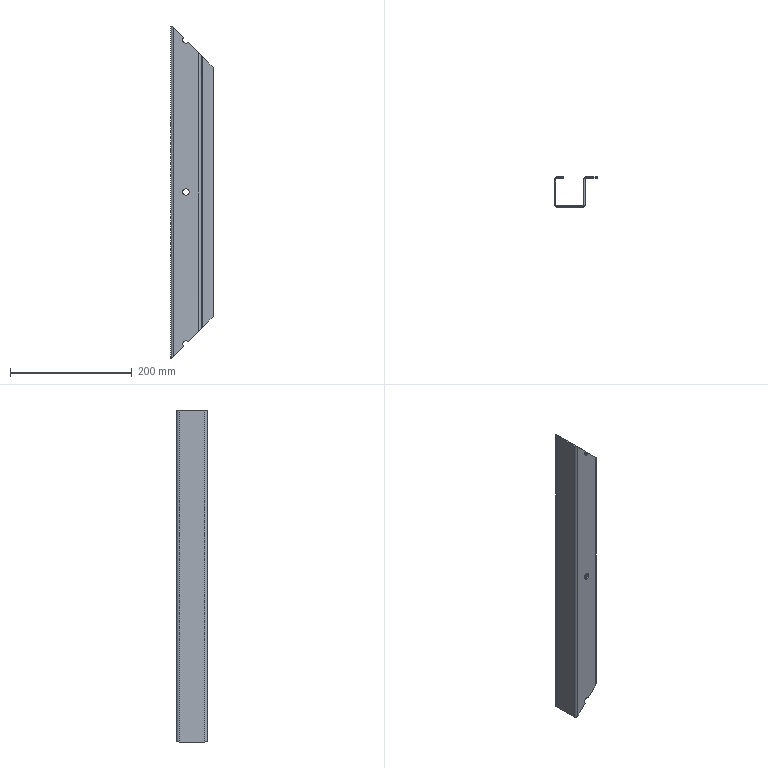Part | STEP file | 750038493 | 1 solid | 45 faces | box 70 x 50 x 546 mm | volume 171168 mm3 | plane 24 | cylinder 13 | spline 8 | commonest cylinder face diameters 10.5 x5 4 x4 8 x4
STEP:
#1=CARTESIAN_POINT('',(25.,2.,5.25));
#2=VERTEX_POINT('',#1);
#3=CARTESIAN_POINT('',(25.,2.,-5.25));
#4=VERTEX_POINT('',#3);
#5=CARTESIAN_POINT('',(25.,2.,0.));
#6=DIRECTION('',(0.,-1.,0.));
#7=DIRECTION('',(0.,0.,-1.));
#8=AXIS2_PLACEMENT_3D('',#5,#6,#7);
#9=CIRCLE('',#8,5.25);
#10=EDGE_CURVE('',#2,#4,#9,.T.);
#11=ORIENTED_EDGE('',*,*,#10,.F.);
#12=CARTESIAN_POINT('',(25.,0.,5.25));
#13=VERTEX_POINT('',#12);
#14=CARTESIAN_POINT('',(25.,552.735,5.25));
#15=DIRECTION('',(0.,-1.,0.));
#16=VECTOR('',#15,1000.);
#17=LINE('',#14,#16);
#18=EDGE_CURVE('',#2,#13,#17,.T.);
#19=ORIENTED_EDGE('',*,*,#18,.T.);
#20=CARTESIAN_POINT('',(25.,0.,-5.25));
#21=VERTEX_POINT('',#20);
#22=CARTESIAN_POINT('',(25.,0.,0.));
#23=DIRECTION('',(0.,1.,0.));
#24=DIRECTION('',(0.,0.,-1.));
#25=AXIS2_PLACEMENT_3D('',#22,#23,#24);
#26=CIRCLE('',#25,5.25);
#27=EDGE_CURVE('',#21,#13,#26,.T.);
#28=ORIENTED_EDGE('',*,*,#27,.F.);
#29=CARTESIAN_POINT('',(25.,552.735,-5.25));
#30=DIRECTION('',(0.,-1.,0.));
#31=VECTOR('',#30,1000.);
#32=LINE('',#29,#31);
#33=EDGE_CURVE('',#4,#21,#32,.T.);
#34=ORIENTED_EDGE('',*,*,#33,.F.);
#35=EDGE_LOOP('',(#11,#19,#28,#34));
#36=FACE_OUTER_BOUND('',#35,.T.);
#37=CARTESIAN_POINT('',(25.,552.735,0.));
#38=DIRECTION('',(0.,-1.,0.));
#39=DIRECTION('',(0.,0.,-1.));
#40=AXIS2_PLACEMENT_3D('',#37,#38,#39);
#41=CYLINDRICAL_SURFACE('',#40,5.25);
#42=ADVANCED_FACE('',(#36),#41,.F.);
#43=CARTESIAN_POINT('',(25.,2.,244.75));
#44=VERTEX_POINT('',#43);
#45=CARTESIAN_POINT('',(28.712,2.,246.288));
#46=VERTEX_POINT('',#45);
#47=CARTESIAN_POINT('',(25.,2.,250.));
#48=DIRECTION('',(0.,-1.,0.));
#49=DIRECTION('',(0.,0.,-1.));
#50=AXIS2_PLACEMENT_3D('',#47,#48,#49);
#51=CIRCLE('',#50,5.25);
#52=EDGE_CURVE('',#44,#46,#51,.T.);
#53=ORIENTED_EDGE('',*,*,#52,.F.);
#54=CARTESIAN_POINT('',(25.,0.,244.75));
#55=VERTEX_POINT('',#54);
#56=CARTESIAN_POINT('',(25.,0.,244.75));
#57=DIRECTION('',(0.,-1.,0.));
#58=VECTOR('',#57,1000.);
#59=LINE('',#56,#58);
#60=EDGE_CURVE('',#44,#55,#59,.T.);
#61=ORIENTED_EDGE('',*,*,#60,.T.);
#62=CARTESIAN_POINT('',(28.712,0.,246.288));
#63=VERTEX_POINT('',#62);
#64=CARTESIAN_POINT('',(25.,0.,250.));
#65=DIRECTION('',(0.,1.,0.));
#66=DIRECTION('',(0.,0.,-1.));
#67=AXIS2_PLACEMENT_3D('',#64,#65,#66);
#68=CIRCLE('',#67,5.25);
#69=EDGE_CURVE('',#63,#55,#68,.T.);
#70=ORIENTED_EDGE('',*,*,#69,.F.);
#71=CARTESIAN_POINT('',(28.712,0.,246.288));
#72=DIRECTION('',(0.,1.,0.));
#73=VECTOR('',#72,1000.);
#74=LINE('',#71,#73);
#75=EDGE_CURVE('',#63,#46,#74,.T.);
#76=ORIENTED_EDGE('',*,*,#75,.T.);
#77=EDGE_LOOP('',(#53,#61,#70,#76));
#78=FACE_OUTER_BOUND('',#77,.T.);
#79=CARTESIAN_POINT('',(25.,0.,250.));
#80=DIRECTION('',(0.,-1.,0.));
#81=DIRECTION('',(0.,0.,-1.));
#82=AXIS2_PLACEMENT_3D('',#79,#80,#81);
#83=CYLINDRICAL_SURFACE('',#82,5.25);
#84=ADVANCED_FACE('',(#78),#83,.F.);
#85=CARTESIAN_POINT('',(0.,46.,-273.));
#86=VERTEX_POINT('',#85);
#87=CARTESIAN_POINT('',(0.,4.,-273.));
#88=VERTEX_POINT('',#87);
#89=CARTESIAN_POINT('',(0.,0.,-273.));
#90=DIRECTION('',(0.,-1.,0.));
#91=VECTOR('',#90,1000.);
#92=LINE('',#89,#91);
#93=EDGE_CURVE('',#86,#88,#92,.T.);
#94=ORIENTED_EDGE('',*,*,#93,.T.);
#95=CARTESIAN_POINT('',(0.,4.,273.));
#96=VERTEX_POINT('',#95);
#97=CARTESIAN_POINT('',(0.,4.,275.));
#98=DIRECTION('',(0.,0.,1.));
#99=VECTOR('',#98,1000.);
#100=LINE('',#97,#99);
#101=EDGE_CURVE('',#88,#96,#100,.T.);
#102=ORIENTED_EDGE('',*,*,#101,.T.);
#103=CARTESIAN_POINT('',(0.,46.,273.));
#104=VERTEX_POINT('',#103);
#105=CARTESIAN_POINT('',(0.,0.,273.));
#106=DIRECTION('',(0.,1.,0.));
#107=VECTOR('',#106,1000.);
#108=LINE('',#105,#107);
#109=EDGE_CURVE('',#96,#104,#108,.T.);
#110=ORIENTED_EDGE('',*,*,#109,.T.);
#111=CARTESIAN_POINT('',(0.,46.,275.));
#112=DIRECTION('',(0.,0.,-1.));
#113=VECTOR('',#112,1000.);
#114=LINE('',#111,#113);
#115=EDGE_CURVE('',#104,#86,#114,.T.);
#116=ORIENTED_EDGE('',*,*,#115,.T.);
#117=EDGE_LOOP('',(#94,#102,#110,#116));
#118=FACE_OUTER_BOUND('',#117,.T.);
#119=CARTESIAN_POINT('',(0.,0.,275.));
#120=DIRECTION('',(-1.,0.,0.));
#121=DIRECTION('',(0.,-1.,0.));
#122=AXIS2_PLACEMENT_3D('',#119,#120,#121);
#123=PLANE('',#122);
#124=ADVANCED_FACE('',(#118),#123,.T.);
#125=CARTESIAN_POINT('',(4.,0.,-271.));
#126=VERTEX_POINT('',#125);
#127=CARTESIAN_POINT('',(0.,4.,-273.));
#128=CARTESIAN_POINT('',(0.,2.,-273.));
#129=CARTESIAN_POINT('',(1.333,0.,-272.333));
#130=CARTESIAN_POINT('',(4.,0.,-271.));
#131=(BOUNDED_CURVE()B_SPLINE_CURVE(3,(#127,#128,#129,#130),.UNSPECIFIED.,.F.,.T.)B_SPLINE_CURVE_WITH_KNOTS((4,4),(0.,0.006692),.UNSPECIFIED.)CURVE()GEOMETRIC_REPRESENTATION_ITEM()RATIONAL_B_SPLINE_CURVE((1.,0.6667,0.5,0.5))REPRESENTATION_ITEM(''));
#132=EDGE_CURVE('',#88,#126,#131,.T.);
#133=ORIENTED_EDGE('',*,*,#132,.T.);
#134=CARTESIAN_POINT('',(4.,0.,271.));
#135=VERTEX_POINT('',#134);
#136=CARTESIAN_POINT('',(4.,0.,275.));
#137=DIRECTION('',(0.,0.,1.));
#138=VECTOR('',#137,1000.);
#139=LINE('',#136,#138);
#140=EDGE_CURVE('',#126,#135,#139,.T.);
#141=ORIENTED_EDGE('',*,*,#140,.T.);
#142=CARTESIAN_POINT('',(4.,0.,271.));
#143=CARTESIAN_POINT('',(1.333,0.,272.333));
#144=CARTESIAN_POINT('',(0.,2.,273.));
#145=CARTESIAN_POINT('',(0.,4.,273.));
#146=(BOUNDED_CURVE()B_SPLINE_CURVE(3,(#142,#143,#144,#145),.UNSPECIFIED.,.F.,.F.)B_SPLINE_CURVE_WITH_KNOTS((4,4),(0.,0.006641),.UNSPECIFIED.)CURVE()GEOMETRIC_REPRESENTATION_ITEM()RATIONAL_B_SPLINE_CURVE((0.5,0.5,0.6667,1.))REPRESENTATION_ITEM(''));
#147=EDGE_CURVE('',#135,#96,#146,.T.);
#148=ORIENTED_EDGE('',*,*,#147,.T.);
#149=ORIENTED_EDGE('',*,*,#101,.F.);
#150=EDGE_LOOP('',(#133,#141,#148,#149));
#151=FACE_OUTER_BOUND('',#150,.T.);
#152=CARTESIAN_POINT('',(4.,4.,275.));
#153=DIRECTION('',(0.,0.,-1.));
#154=DIRECTION('',(-1.,0.,0.));
#155=AXIS2_PLACEMENT_3D('',#152,#153,#154);
#156=CYLINDRICAL_SURFACE('',#155,4.);
#157=ADVANCED_FACE('',(#151),#156,.T.);
#158=CARTESIAN_POINT('',(2.,46.,-273.));
#159=VERTEX_POINT('',#158);
#160=CARTESIAN_POINT('',(2.,46.,-273.));
#161=DIRECTION('',(-1.,0.,0.));
#162=VECTOR('',#161,1000.);
#163=LINE('',#160,#162);
#164=EDGE_CURVE('',#159,#86,#163,.T.);
#165=ORIENTED_EDGE('',*,*,#164,.F.);
#166=CARTESIAN_POINT('',(2.,4.,-273.));
#167=VERTEX_POINT('',#166);
#168=CARTESIAN_POINT('',(2.,0.,-273.));
#169=DIRECTION('',(0.,1.,0.));
#170=VECTOR('',#169,1000.);
#171=LINE('',#168,#170);
#172=EDGE_CURVE('',#167,#159,#171,.T.);
#173=ORIENTED_EDGE('',*,*,#172,.F.);
#174=CARTESIAN_POINT('',(2.,4.,-273.));
#175=DIRECTION('',(1.,0.,0.));
#176=VECTOR('',#175,1000.);
#177=LINE('',#174,#176);
#178=EDGE_CURVE('',#88,#167,#177,.T.);
#179=ORIENTED_EDGE('',*,*,#178,.F.);
#180=ORIENTED_EDGE('',*,*,#93,.F.);
#181=EDGE_LOOP('',(#165,#173,#179,#180));
#182=FACE_OUTER_BOUND('',#181,.T.);
#183=CARTESIAN_POINT('',(2.,0.,-273.));
#184=DIRECTION('',(0.,0.,1.));
#185=DIRECTION('',(0.,-1.,0.));
#186=AXIS2_PLACEMENT_3D('',#183,#184,#185);
#187=PLANE('',#186);
#188=ADVANCED_FACE('',(#182),#187,.F.);
#189=CARTESIAN_POINT('',(4.,50.,-271.));
#190=VERTEX_POINT('',#189);
#191=CARTESIAN_POINT('',(4.,50.,-271.));
#192=CARTESIAN_POINT('',(1.333,50.,-272.333));
#193=CARTESIAN_POINT('',(0.,48.,-273.));
#194=CARTESIAN_POINT('',(0.,46.,-273.));
#195=(BOUNDED_CURVE()B_SPLINE_CURVE(3,(#191,#192,#193,#194),.UNSPECIFIED.,.F.,.F.)B_SPLINE_CURVE_WITH_KNOTS((4,4),(0.,0.006641),.UNSPECIFIED.)CURVE()GEOMETRIC_REPRESENTATION_ITEM()RATIONAL_B_SPLINE_CURVE((0.5,0.5,0.6667,1.))REPRESENTATION_ITEM(''));
#196=EDGE_CURVE('',#190,#86,#195,.T.);
#197=ORIENTED_EDGE('',*,*,#196,.T.);
#198=ORIENTED_EDGE('',*,*,#115,.F.);
#199=CARTESIAN_POINT('',(4.,50.,271.));
#200=VERTEX_POINT('',#199);
#201=CARTESIAN_POINT('',(0.,46.,273.));
#202=CARTESIAN_POINT('',(0.,48.,273.));
#203=CARTESIAN_POINT('',(1.333,50.,272.333));
#204=CARTESIAN_POINT('',(4.,50.,271.));
#205=(BOUNDED_CURVE()B_SPLINE_CURVE(3,(#201,#202,#203,#204),.UNSPECIFIED.,.F.,.F.)B_SPLINE_CURVE_WITH_KNOTS((4,4),(0.,0.006627),.UNSPECIFIED.)CURVE()GEOMETRIC_REPRESENTATION_ITEM()RATIONAL_B_SPLINE_CURVE((1.,0.6667,0.5,0.5))REPRESENTATION_ITEM(''));
#206=EDGE_CURVE('',#104,#200,#205,.T.);
#207=ORIENTED_EDGE('',*,*,#206,.T.);
#208=CARTESIAN_POINT('',(4.,50.,275.));
#209=DIRECTION('',(0.,0.,-1.));
#210=VECTOR('',#209,1000.);
#211=LINE('',#208,#210);
#212=EDGE_CURVE('',#200,#190,#211,.T.);
#213=ORIENTED_EDGE('',*,*,#212,.T.);
#214=EDGE_LOOP('',(#197,#198,#207,#213));
#215=FACE_OUTER_BOUND('',#214,.T.);
#216=CARTESIAN_POINT('',(4.,46.,275.));
#217=DIRECTION('',(0.,0.,-1.));
#218=DIRECTION('',(-1.,0.,0.));
#219=AXIS2_PLACEMENT_3D('',#216,#217,#218);
#220=CYLINDRICAL_SURFACE('',#219,4.);
#221=ADVANCED_FACE('',(#215),#220,.T.);
#222=CARTESIAN_POINT('',(2.,46.,273.));
#223=VERTEX_POINT('',#222);
#224=CARTESIAN_POINT('',(2.,4.,273.));
#225=VERTEX_POINT('',#224);
#226=CARTESIAN_POINT('',(2.,0.,273.));
#227=DIRECTION('',(0.,-1.,0.));
#228=VECTOR('',#227,1000.);
#229=LINE('',#226,#228);
#230=EDGE_CURVE('',#223,#225,#229,.T.);
#231=ORIENTED_EDGE('',*,*,#230,.F.);
#232=CARTESIAN_POINT('',(2.,46.,273.));
#233=DIRECTION('',(1.,0.,0.));
#234=VECTOR('',#233,1000.);
#235=LINE('',#232,#234);
#236=EDGE_CURVE('',#104,#223,#235,.T.);
#237=ORIENTED_EDGE('',*,*,#236,.F.);
#238=ORIENTED_EDGE('',*,*,#109,.F.);
#239=CARTESIAN_POINT('',(2.,4.,273.));
#240=DIRECTION('',(-1.,0.,0.));
#241=VECTOR('',#240,1000.);
#242=LINE('',#239,#241);
#243=EDGE_CURVE('',#225,#96,#242,.T.);
#244=ORIENTED_EDGE('',*,*,#243,.F.);
#245=EDGE_LOOP('',(#231,#237,#238,#244));
#246=FACE_OUTER_BOUND('',#245,.T.);
#247=CARTESIAN_POINT('',(2.,0.,273.));
#248=DIRECTION('',(0.,0.,-1.));
#249=DIRECTION('',(0.,1.,0.));
#250=AXIS2_PLACEMENT_3D('',#247,#248,#249);
#251=PLANE('',#250);
#252=ADVANCED_FACE('',(#246),#251,.F.);
#253=ORIENTED_EDGE('',*,*,#27,.T.);
#254=CARTESIAN_POINT('',(25.,0.,0.));
#255=DIRECTION('',(0.,1.,0.));
#256=DIRECTION('',(0.,0.,-1.));
#257=AXIS2_PLACEMENT_3D('',#254,#255,#256);
#258=CIRCLE('',#257,5.25);
#259=EDGE_CURVE('',#13,#21,#258,.T.);
#260=ORIENTED_EDGE('',*,*,#259,.T.);
#261=EDGE_LOOP('',(#253,#260));
#262=FACE_BOUND('',#261,.T.);
#263=CARTESIAN_POINT('',(46.,0.,-229.));
#264=VERTEX_POINT('',#263);
#265=CARTESIAN_POINT('',(46.,0.,229.));
#266=VERTEX_POINT('',#265);
#267=CARTESIAN_POINT('',(46.,0.,275.));
#268=DIRECTION('',(0.,0.,1.));
#269=VECTOR('',#268,1000.);
#270=LINE('',#267,#269);
#271=EDGE_CURVE('',#264,#266,#270,.T.);
#272=ORIENTED_EDGE('',*,*,#271,.T.);
#273=CARTESIAN_POINT('',(46.,0.,229.));
#274=DIRECTION('',(-0.7071,0.,0.7071));
#275=VECTOR('',#274,1000.);
#276=LINE('',#273,#275);
#277=EDGE_CURVE('',#266,#63,#276,.T.);
#278=ORIENTED_EDGE('',*,*,#277,.T.);
#279=ORIENTED_EDGE('',*,*,#69,.T.);
#280=CARTESIAN_POINT('',(21.288,0.,253.712));
#281=VERTEX_POINT('',#280);
#282=CARTESIAN_POINT('',(25.,0.,250.));
#283=DIRECTION('',(0.,1.,0.));
#284=DIRECTION('',(0.,0.,-1.));
#285=AXIS2_PLACEMENT_3D('',#282,#283,#284);
#286=CIRCLE('',#285,5.25);
#287=EDGE_CURVE('',#55,#281,#286,.T.);
#288=ORIENTED_EDGE('',*,*,#287,.T.);
#289=CARTESIAN_POINT('',(21.288,0.,253.712));
#290=DIRECTION('',(-0.7071,0.,0.7071));
#291=VECTOR('',#290,1000.);
#292=LINE('',#289,#291);
#293=EDGE_CURVE('',#281,#135,#292,.T.);
#294=ORIENTED_EDGE('',*,*,#293,.T.);
#295=ORIENTED_EDGE('',*,*,#140,.F.);
#296=CARTESIAN_POINT('',(21.288,0.,-253.712));
#297=VERTEX_POINT('',#296);
#298=CARTESIAN_POINT('',(4.,0.,-271.));
#299=DIRECTION('',(0.7071,0.,0.7071));
#300=VECTOR('',#299,1000.);
#301=LINE('',#298,#300);
#302=EDGE_CURVE('',#126,#297,#301,.T.);
#303=ORIENTED_EDGE('',*,*,#302,.T.);
#304=CARTESIAN_POINT('',(28.712,0.,-246.288));
#305=VERTEX_POINT('',#304);
#306=CARTESIAN_POINT('',(25.,0.,-250.));
#307=DIRECTION('',(0.,1.,0.));
#308=DIRECTION('',(0.,0.,-1.));
#309=AXIS2_PLACEMENT_3D('',#306,#307,#308);
#310=CIRCLE('',#309,5.25);
#311=EDGE_CURVE('',#297,#305,#310,.T.);
#312=ORIENTED_EDGE('',*,*,#311,.T.);
#313=CARTESIAN_POINT('',(28.712,0.,-246.288));
#314=DIRECTION('',(0.7071,0.,0.7071));
#315=VECTOR('',#314,1000.);
#316=LINE('',#313,#315);
#317=EDGE_CURVE('',#305,#264,#316,.T.);
#318=ORIENTED_EDGE('',*,*,#317,.T.);
#319=EDGE_LOOP('',(#272,#278,#279,#288,#294,#295,#303,#312,#318));
#320=FACE_OUTER_BOUND('',#319,.T.);
#321=CARTESIAN_POINT('',(50.,0.,275.));
#322=DIRECTION('',(0.,-1.,0.));
#323=DIRECTION('',(0.,0.,-1.));
#324=AXIS2_PLACEMENT_3D('',#321,#322,#323);
#325=PLANE('',#324);
#326=ADVANCED_FACE('',(#262,#320),#325,.T.);
#327=CARTESIAN_POINT('',(4.,2.,-271.));
#328=VERTEX_POINT('',#327);
#329=CARTESIAN_POINT('',(4.,1.,-271.));
#330=DIRECTION('',(0.,-1.,0.));
#331=VECTOR('',#330,1000.);
#332=LINE('',#329,#331);
#333=EDGE_CURVE('',#328,#126,#332,.T.);
#334=ORIENTED_EDGE('',*,*,#333,.T.);
#335=ORIENTED_EDGE('',*,*,#132,.F.);
#336=ORIENTED_EDGE('',*,*,#178,.T.);
#337=CARTESIAN_POINT('',(2.,4.,-273.));
#338=CARTESIAN_POINT('',(2.,3.,-273.));
#339=CARTESIAN_POINT('',(2.667,2.,-272.333));
#340=CARTESIAN_POINT('',(4.,2.,-271.));
#341=(BOUNDED_CURVE()B_SPLINE_CURVE(3,(#337,#338,#339,#340),.UNSPECIFIED.,.F.,.F.)B_SPLINE_CURVE_WITH_KNOTS((4,4),(0.,0.003854),.UNSPECIFIED.)CURVE()GEOMETRIC_REPRESENTATION_ITEM()RATIONAL_B_SPLINE_CURVE((1.,0.6667,0.5,0.5))REPRESENTATION_ITEM(''));
#342=EDGE_CURVE('',#167,#328,#341,.T.);
#343=ORIENTED_EDGE('',*,*,#342,.T.);
#344=EDGE_LOOP('',(#334,#335,#336,#343));
#345=FACE_OUTER_BOUND('',#344,.T.);
#346=CARTESIAN_POINT('',(0.,4.,-273.));
#347=CARTESIAN_POINT('',(0.6667,4.,-273.));
#348=CARTESIAN_POINT('',(1.333,4.,-273.));
#349=CARTESIAN_POINT('',(2.,4.,-273.));
#350=CARTESIAN_POINT('',(0.,12.,-273.));
#351=CARTESIAN_POINT('',(0.6667,10.667,-273.));
#352=CARTESIAN_POINT('',(1.333,9.333,-273.));
#353=CARTESIAN_POINT('',(2.,8.,-273.));
#354=CARTESIAN_POINT('',(8.,12.,-269.));
#355=CARTESIAN_POINT('',(7.333,10.667,-269.));
#356=CARTESIAN_POINT('',(6.667,9.333,-269.));
#357=CARTESIAN_POINT('',(6.,8.,-269.));
#358=CARTESIAN_POINT('',(8.,4.,-269.));
#359=CARTESIAN_POINT('',(7.333,4.,-269.));
#360=CARTESIAN_POINT('',(6.667,4.,-269.));
#361=CARTESIAN_POINT('',(6.,4.,-269.));
#362=CARTESIAN_POINT('',(8.,-4.,-269.));
#363=CARTESIAN_POINT('',(7.333,-2.667,-269.));
#364=CARTESIAN_POINT('',(6.667,-1.333,-269.));
#365=CARTESIAN_POINT('',(6.,0.,-269.));
#366=CARTESIAN_POINT('',(0.,-4.,-273.));
#367=CARTESIAN_POINT('',(0.6667,-2.667,-273.));
#368=CARTESIAN_POINT('',(1.333,-1.333,-273.));
#369=CARTESIAN_POINT('',(2.,0.,-273.));
#370=CARTESIAN_POINT('',(0.,4.,-273.));
#371=CARTESIAN_POINT('',(0.6667,4.,-273.));
#372=CARTESIAN_POINT('',(1.333,4.,-273.));
#373=CARTESIAN_POINT('',(2.,4.,-273.));
#374=(BOUNDED_SURFACE()B_SPLINE_SURFACE(3,3,((#346,#347,#348,#349),(#350,#351,#352,#353),(#354,#355,#356,#357),(#358,#359,#360,#361),(#362,#363,#364,#365),(#366,#367,#368,#369),(#370,#371,#372,#373)),.UNSPECIFIED.,.T.,.F.,.T.)B_SPLINE_SURFACE_WITH_KNOTS((4,3,4),(4,4),(0.,0.5,1.),(0.,1.),.UNSPECIFIED.)GEOMETRIC_REPRESENTATION_ITEM()RATIONAL_B_SPLINE_SURFACE(((1.,1.,1.,1.),(0.3333,0.3333,0.3333,0.3333),(0.3333,0.3333,0.3333,0.3333),(1.,1.,1.,1.),(0.3333,0.3333,0.3333,0.3333),(0.3333,0.3333,0.3333,0.3333),(1.,1.,1.,1.)))REPRESENTATION_ITEM('')SURFACE());
#375=ADVANCED_FACE('',(#345),#374,.T.);
#376=ORIENTED_EDGE('',*,*,#243,.T.);
#377=ORIENTED_EDGE('',*,*,#147,.F.);
#378=CARTESIAN_POINT('',(4.,2.,271.));
#379=VERTEX_POINT('',#378);
#380=CARTESIAN_POINT('',(4.,1.,271.));
#381=DIRECTION('',(0.,1.,0.));
#382=VECTOR('',#381,1000.);
#383=LINE('',#380,#382);
#384=EDGE_CURVE('',#135,#379,#383,.T.);
#385=ORIENTED_EDGE('',*,*,#384,.T.);
#386=CARTESIAN_POINT('',(4.,2.,271.));
#387=CARTESIAN_POINT('',(2.667,2.,272.333));
#388=CARTESIAN_POINT('',(2.,3.,273.));
#389=CARTESIAN_POINT('',(2.,4.,273.));
#390=(BOUNDED_CURVE()B_SPLINE_CURVE(3,(#386,#387,#388,#389),.UNSPECIFIED.,.F.,.F.)B_SPLINE_CURVE_WITH_KNOTS((4,4),(0.,0.003785),.UNSPECIFIED.)CURVE()GEOMETRIC_REPRESENTATION_ITEM()RATIONAL_B_SPLINE_CURVE((0.5,0.5,0.6667,1.))REPRESENTATION_ITEM(''));
#391=EDGE_CURVE('',#379,#225,#390,.T.);
#392=ORIENTED_EDGE('',*,*,#391,.T.);
#393=EDGE_LOOP('',(#376,#377,#385,#392));
#394=FACE_OUTER_BOUND('',#393,.T.);
#395=CARTESIAN_POINT('',(8.,4.,269.));
#396=CARTESIAN_POINT('',(7.333,4.,269.));
#397=CARTESIAN_POINT('',(6.667,4.,269.));
#398=CARTESIAN_POINT('',(6.,4.,269.));
#399=CARTESIAN_POINT('',(8.,12.,269.));
#400=CARTESIAN_POINT('',(7.333,10.667,269.));
#401=CARTESIAN_POINT('',(6.667,9.333,269.));
#402=CARTESIAN_POINT('',(6.,8.,269.));
#403=CARTESIAN_POINT('',(0.,12.,273.));
#404=CARTESIAN_POINT('',(0.6667,10.667,273.));
#405=CARTESIAN_POINT('',(1.333,9.333,273.));
#406=CARTESIAN_POINT('',(2.,8.,273.));
#407=CARTESIAN_POINT('',(0.,4.,273.));
#408=CARTESIAN_POINT('',(0.6667,4.,273.));
#409=CARTESIAN_POINT('',(1.333,4.,273.));
#410=CARTESIAN_POINT('',(2.,4.,273.));
#411=CARTESIAN_POINT('',(0.,-4.,273.));
#412=CARTESIAN_POINT('',(0.6667,-2.667,273.));
#413=CARTESIAN_POINT('',(1.333,-1.333,273.));
#414=CARTESIAN_POINT('',(2.,0.,273.));
#415=CARTESIAN_POINT('',(8.,-4.,269.));
#416=CARTESIAN_POINT('',(7.333,-2.667,269.));
#417=CARTESIAN_POINT('',(6.667,-1.333,269.));
#418=CARTESIAN_POINT('',(6.,0.,269.));
#419=CARTESIAN_POINT('',(8.,4.,269.));
#420=CARTESIAN_POINT('',(7.333,4.,269.));
#421=CARTESIAN_POINT('',(6.667,4.,269.));
#422=CARTESIAN_POINT('',(6.,4.,269.));
#423=(BOUNDED_SURFACE()B_SPLINE_SURFACE(3,3,((#395,#396,#397,#398),(#399,#400,#401,#402),(#403,#404,#405,#406),(#407,#408,#409,#410),(#411,#412,#413,#414),(#415,#416,#417,#418),(#419,#420,#421,#422)),.UNSPECIFIED.,.T.,.F.,.F.)B_SPLINE_SURFACE_WITH_KNOTS((4,3,4),(4,4),(0.,0.5,1.),(0.,1.),.UNSPECIFIED.)GEOMETRIC_REPRESENTATION_ITEM()RATIONAL_B_SPLINE_SURFACE(((1.,1.,1.,1.),(0.3333,0.3333,0.3333,0.3333),(0.3333,0.3333,0.3333,0.3333),(1.,1.,1.,1.),(0.3333,0.3333,0.3333,0.3333),(0.3333,0.3333,0.3333,0.3333),(1.,1.,1.,1.)))REPRESENTATION_ITEM('')SURFACE());
#424=ADVANCED_FACE('',(#394),#423,.T.);
#425=ORIENTED_EDGE('',*,*,#164,.T.);
#426=ORIENTED_EDGE('',*,*,#196,.F.);
#427=CARTESIAN_POINT('',(4.,48.,-271.));
#428=VERTEX_POINT('',#427);
#429=CARTESIAN_POINT('',(4.,49.,-271.));
#430=DIRECTION('',(0.,-1.,0.));
#431=VECTOR('',#430,1000.);
#432=LINE('',#429,#431);
#433=EDGE_CURVE('',#190,#428,#432,.T.);
#434=ORIENTED_EDGE('',*,*,#433,.T.);
#435=CARTESIAN_POINT('',(4.,48.,-271.));
#436=CARTESIAN_POINT('',(2.667,48.,-272.333));
#437=CARTESIAN_POINT('',(2.,47.,-273.));
#438=CARTESIAN_POINT('',(2.,46.,-273.));
#439=(BOUNDED_CURVE()B_SPLINE_CURVE(3,(#435,#436,#437,#438),.UNSPECIFIED.,.F.,.F.)B_SPLINE_CURVE_WITH_KNOTS((4,4),(0.,0.003785),.UNSPECIFIED.)CURVE()GEOMETRIC_REPRESENTATION_ITEM()RATIONAL_B_SPLINE_CURVE((0.5,0.5,0.6667,1.))REPRESENTATION_ITEM(''));
#440=EDGE_CURVE('',#428,#159,#439,.T.);
#441=ORIENTED_EDGE('',*,*,#440,.T.);
#442=EDGE_LOOP('',(#425,#426,#434,#441));
#443=FACE_OUTER_BOUND('',#442,.T.);
#444=CARTESIAN_POINT('',(0.,46.,-273.));
#445=CARTESIAN_POINT('',(0.6667,46.,-273.));
#446=CARTESIAN_POINT('',(1.333,46.,-273.));
#447=CARTESIAN_POINT('',(2.,46.,-273.));
#448=CARTESIAN_POINT('',(0.,54.,-273.));
#449=CARTESIAN_POINT('',(0.6667,52.667,-273.));
#450=CARTESIAN_POINT('',(1.333,51.333,-273.));
#451=CARTESIAN_POINT('',(2.,50.,-273.));
#452=CARTESIAN_POINT('',(8.,54.,-269.));
#453=CARTESIAN_POINT('',(7.333,52.667,-269.));
#454=CARTESIAN_POINT('',(6.667,51.333,-269.));
#455=CARTESIAN_POINT('',(6.,50.,-269.));
#456=CARTESIAN_POINT('',(8.,46.,-269.));
#457=CARTESIAN_POINT('',(7.333,46.,-269.));
#458=CARTESIAN_POINT('',(6.667,46.,-269.));
#459=CARTESIAN_POINT('',(6.,46.,-269.));
#460=CARTESIAN_POINT('',(8.,38.,-269.));
#461=CARTESIAN_POINT('',(7.333,39.333,-269.));
#462=CARTESIAN_POINT('',(6.667,40.667,-269.));
#463=CARTESIAN_POINT('',(6.,42.,-269.));
#464=CARTESIAN_POINT('',(0.,38.,-273.));
#465=CARTESIAN_POINT('',(0.6667,39.333,-273.));
#466=CARTESIAN_POINT('',(1.333,40.667,-273.));
#467=CARTESIAN_POINT('',(2.,42.,-273.));
#468=CARTESIAN_POINT('',(0.,46.,-273.));
#469=CARTESIAN_POINT('',(0.6667,46.,-273.));
#470=CARTESIAN_POINT('',(1.333,46.,-273.));
#471=CARTESIAN_POINT('',(2.,46.,-273.));
#472=(BOUNDED_SURFACE()B_SPLINE_SURFACE(3,3,((#444,#445,#446,#447),(#448,#449,#450,#451),(#452,#453,#454,#455),(#456,#457,#458,#459),(#460,#461,#462,#463),(#464,#465,#466,#467),(#468,#469,#470,#471)),.UNSPECIFIED.,.T.,.F.,.F.)B_SPLINE_SURFACE_WITH_KNOTS((4,3,4),(4,4),(0.,0.5,1.),(0.,1.),.UNSPECIFIED.)GEOMETRIC_REPRESENTATION_ITEM()RATIONAL_B_SPLINE_SURFACE(((1.,1.,1.,1.),(0.3333,0.3333,0.3333,0.3333),(0.3333,0.3333,0.3333,0.3333),(1.,1.,1.,1.),(0.3333,0.3333,0.3333,0.3333),(0.3333,0.3333,0.3333,0.3333),(1.,1.,1.,1.)))REPRESENTATION_ITEM('')SURFACE());
#473=ADVANCED_FACE('',(#443),#472,.T.);
#474=ORIENTED_EDGE('',*,*,#230,.T.);
#475=CARTESIAN_POINT('',(2.,4.,275.));
#476=DIRECTION('',(0.,0.,1.));
#477=VECTOR('',#476,1000.);
#478=LINE('',#475,#477);
#479=EDGE_CURVE('',#167,#225,#478,.T.);
#480=ORIENTED_EDGE('',*,*,#479,.F.);
#481=ORIENTED_EDGE('',*,*,#172,.T.);
#482=CARTESIAN_POINT('',(2.,46.,275.));
#483=DIRECTION('',(0.,0.,-1.));
#484=VECTOR('',#483,1000.);
#485=LINE('',#482,#484);
#486=EDGE_CURVE('',#223,#159,#485,.T.);
#487=ORIENTED_EDGE('',*,*,#486,.F.);
#488=EDGE_LOOP('',(#474,#480,#481,#487));
#489=FACE_OUTER_BOUND('',#488,.T.);
#490=CARTESIAN_POINT('',(2.,0.,275.));
#491=DIRECTION('',(-1.,0.,0.));
#492=DIRECTION('',(0.,-1.,0.));
#493=AXIS2_PLACEMENT_3D('',#490,#491,#492);
#494=PLANE('',#493);
#495=ADVANCED_FACE('',(#489),#494,.F.);
#496=CARTESIAN_POINT('',(15.,50.,-260.));
#497=VERTEX_POINT('',#496);
#498=CARTESIAN_POINT('',(15.,50.,-260.));
#499=DIRECTION('',(-0.7071,0.,-0.7071));
#500=VECTOR('',#499,1000.);
#501=LINE('',#498,#500);
#502=EDGE_CURVE('',#497,#190,#501,.T.);
#503=ORIENTED_EDGE('',*,*,#502,.T.);
#504=ORIENTED_EDGE('',*,*,#212,.F.);
#505=CARTESIAN_POINT('',(15.,50.,260.));
#506=VERTEX_POINT('',#505);
#507=CARTESIAN_POINT('',(4.,50.,271.));
#508=DIRECTION('',(0.7071,0.,-0.7071));
#509=VECTOR('',#508,1000.);
#510=LINE('',#507,#509);
#511=EDGE_CURVE('',#200,#506,#510,.T.);
#512=ORIENTED_EDGE('',*,*,#511,.T.);
#513=CARTESIAN_POINT('',(15.,50.,275.));
#514=DIRECTION('',(0.,0.,-1.));
#515=VECTOR('',#514,1000.);
#516=LINE('',#513,#515);
#517=EDGE_CURVE('',#506,#497,#516,.T.);
#518=ORIENTED_EDGE('',*,*,#517,.T.);
#519=EDGE_LOOP('',(#503,#504,#512,#518));
#520=FACE_OUTER_BOUND('',#519,.T.);
#521=CARTESIAN_POINT('',(0.,50.,275.));
#522=DIRECTION('',(0.,1.,0.));
#523=DIRECTION('',(0.,0.,1.));
#524=AXIS2_PLACEMENT_3D('',#521,#522,#523);
#525=PLANE('',#524);
#526=ADVANCED_FACE('',(#520),#525,.T.);
#527=CARTESIAN_POINT('',(4.,48.,271.));
#528=VERTEX_POINT('',#527);
#529=CARTESIAN_POINT('',(4.,49.,271.));
#530=DIRECTION('',(0.,1.,0.));
#531=VECTOR('',#530,1000.);
#532=LINE('',#529,#531);
#533=EDGE_CURVE('',#528,#200,#532,.T.);
#534=ORIENTED_EDGE('',*,*,#533,.T.);
#535=ORIENTED_EDGE('',*,*,#206,.F.);
#536=ORIENTED_EDGE('',*,*,#236,.T.);
#537=CARTESIAN_POINT('',(2.,46.,273.));
#538=CARTESIAN_POINT('',(2.,47.,273.));
#539=CARTESIAN_POINT('',(2.667,48.,272.333));
#540=CARTESIAN_POINT('',(4.,48.,271.));
#541=(BOUNDED_CURVE()B_SPLINE_CURVE(3,(#537,#538,#539,#540),.UNSPECIFIED.,.F.,.F.)B_SPLINE_CURVE_WITH_KNOTS((4,4),(0.,0.003806),.UNSPECIFIED.)CURVE()GEOMETRIC_REPRESENTATION_ITEM()RATIONAL_B_SPLINE_CURVE((1.,0.6667,0.5,0.5))REPRESENTATION_ITEM(''));
#542=EDGE_CURVE('',#223,#528,#541,.T.);
#543=ORIENTED_EDGE('',*,*,#542,.T.);
#544=EDGE_LOOP('',(#534,#535,#536,#543));
#545=FACE_OUTER_BOUND('',#544,.T.);
#546=CARTESIAN_POINT('',(8.,46.,269.));
#547=CARTESIAN_POINT('',(7.333,46.,269.));
#548=CARTESIAN_POINT('',(6.667,46.,269.));
#549=CARTESIAN_POINT('',(6.,46.,269.));
#550=CARTESIAN_POINT('',(8.,54.,269.));
#551=CARTESIAN_POINT('',(7.333,52.667,269.));
#552=CARTESIAN_POINT('',(6.667,51.333,269.));
#553=CARTESIAN_POINT('',(6.,50.,269.));
#554=CARTESIAN_POINT('',(0.,54.,273.));
#555=CARTESIAN_POINT('',(0.6667,52.667,273.));
#556=CARTESIAN_POINT('',(1.333,51.333,273.));
#557=CARTESIAN_POINT('',(2.,50.,273.));
#558=CARTESIAN_POINT('',(0.,46.,273.));
#559=CARTESIAN_POINT('',(0.6667,46.,273.));
#560=CARTESIAN_POINT('',(1.333,46.,273.));
#561=CARTESIAN_POINT('',(2.,46.,273.));
#562=CARTESIAN_POINT('',(0.,38.,273.));
#563=CARTESIAN_POINT('',(0.6667,39.333,273.));
#564=CARTESIAN_POINT('',(1.333,40.667,273.));
#565=CARTESIAN_POINT('',(2.,42.,273.));
#566=CARTESIAN_POINT('',(8.,38.,269.));
#567=CARTESIAN_POINT('',(7.333,39.333,269.));
#568=CARTESIAN_POINT('',(6.667,40.667,269.));
#569=CARTESIAN_POINT('',(6.,42.,269.));
#570=CARTESIAN_POINT('',(8.,46.,269.));
#571=CARTESIAN_POINT('',(7.333,46.,269.));
#572=CARTESIAN_POINT('',(6.667,46.,269.));
#573=CARTESIAN_POINT('',(6.,46.,269.));
#574=(BOUNDED_SURFACE()B_SPLINE_SURFACE(3,3,((#546,#547,#548,#549),(#550,#551,#552,#553),(#554,#555,#556,#557),(#558,#559,#560,#561),(#562,#563,#564,#565),(#566,#567,#568,#569),(#570,#571,#572,#573)),.UNSPECIFIED.,.T.,.F.,.F.)B_SPLINE_SURFACE_WITH_KNOTS((4,3,4),(4,4),(0.,0.5,1.),(0.,1.),.UNSPECIFIED.)GEOMETRIC_REPRESENTATION_ITEM()RATIONAL_B_SPLINE_SURFACE(((1.,1.,1.,1.),(0.3333,0.3333,0.3333,0.3333),(0.3333,0.3333,0.3333,0.3333),(1.,1.,1.,1.),(0.3333,0.3333,0.3333,0.3333),(0.3333,0.3333,0.3333,0.3333),(1.,1.,1.,1.)))REPRESENTATION_ITEM('')SURFACE());
#575=ADVANCED_FACE('',(#545),#574,.T.);
#576=ORIENTED_EDGE('',*,*,#18,.F.);
#577=CARTESIAN_POINT('',(25.,2.,0.));
#578=DIRECTION('',(0.,-1.,0.));
#579=DIRECTION('',(0.,0.,-1.));
#580=AXIS2_PLACEMENT_3D('',#577,#578,#579);
#581=CIRCLE('',#580,5.25);
#582=EDGE_CURVE('',#4,#2,#581,.T.);
#583=ORIENTED_EDGE('',*,*,#582,.F.);
#584=ORIENTED_EDGE('',*,*,#33,.T.);
#585=ORIENTED_EDGE('',*,*,#259,.F.);
#586=EDGE_LOOP('',(#576,#583,#584,#585));
#587=FACE_OUTER_BOUND('',#586,.T.);
#588=CARTESIAN_POINT('',(25.,552.735,0.));
#589=DIRECTION('',(0.,-1.,0.));
#590=DIRECTION('',(0.,0.,-1.));
#591=AXIS2_PLACEMENT_3D('',#588,#589,#590);
#592=CYLINDRICAL_SURFACE('',#591,5.25);
#593=ADVANCED_FACE('',(#587),#592,.F.);
#594=ORIENTED_EDGE('',*,*,#75,.F.);
#595=ORIENTED_EDGE('',*,*,#277,.F.);
#596=CARTESIAN_POINT('',(46.,2.,229.));
#597=VERTEX_POINT('',#596);
#598=CARTESIAN_POINT('',(46.,0.,229.));
#599=DIRECTION('',(0.,-1.,0.));
#600=VECTOR('',#599,1000.);
#601=LINE('',#598,#600);
#602=EDGE_CURVE('',#597,#266,#601,.T.);
#603=ORIENTED_EDGE('',*,*,#602,.F.);
#604=CARTESIAN_POINT('',(25.,2.,250.));
#605=DIRECTION('',(0.7071,0.,-0.7071));
#606=VECTOR('',#605,1000.);
#607=LINE('',#604,#606);
#608=EDGE_CURVE('',#46,#597,#607,.T.);
#609=ORIENTED_EDGE('',*,*,#608,.F.);
#610=EDGE_LOOP('',(#594,#595,#603,#609));
#611=FACE_OUTER_BOUND('',#610,.T.);
#612=CARTESIAN_POINT('',(25.,0.,250.));
#613=DIRECTION('',(-0.7071,0.,-0.7071));
#614=DIRECTION('',(-0.7071,0.,0.7071));
#615=AXIS2_PLACEMENT_3D('',#612,#613,#614);
#616=PLANE('',#615);
#617=ADVANCED_FACE('',(#611),#616,.F.);
#618=CARTESIAN_POINT('',(50.,4.,-225.));
#619=VERTEX_POINT('',#618);
#620=CARTESIAN_POINT('',(46.,0.,-229.));
#621=CARTESIAN_POINT('',(48.667,0.,-226.333));
#622=CARTESIAN_POINT('',(50.,2.,-225.));
#623=CARTESIAN_POINT('',(50.,4.,-225.));
#624=(BOUNDED_CURVE()B_SPLINE_CURVE(3,(#620,#621,#622,#623),.UNSPECIFIED.,.F.,.F.)B_SPLINE_CURVE_WITH_KNOTS((4,4),(0.,0.007567),.UNSPECIFIED.)CURVE()GEOMETRIC_REPRESENTATION_ITEM()RATIONAL_B_SPLINE_CURVE((0.5,0.5,0.6667,1.))REPRESENTATION_ITEM(''));
#625=EDGE_CURVE('',#264,#619,#624,.T.);
#626=ORIENTED_EDGE('',*,*,#625,.T.);
#627=CARTESIAN_POINT('',(50.,4.,225.));
#628=VERTEX_POINT('',#627);
#629=CARTESIAN_POINT('',(50.,4.,275.));
#630=DIRECTION('',(0.,0.,1.));
#631=VECTOR('',#630,1000.);
#632=LINE('',#629,#631);
#633=EDGE_CURVE('',#619,#628,#632,.T.);
#634=ORIENTED_EDGE('',*,*,#633,.T.);
#635=CARTESIAN_POINT('',(50.,4.,225.));
#636=CARTESIAN_POINT('',(50.,2.,225.));
#637=CARTESIAN_POINT('',(48.667,0.,226.333));
#638=CARTESIAN_POINT('',(46.,0.,229.));
#639=(BOUNDED_CURVE()B_SPLINE_CURVE(3,(#635,#636,#637,#638),.UNSPECIFIED.,.F.,.F.)B_SPLINE_CURVE_WITH_KNOTS((4,4),(0.,0.007712),.UNSPECIFIED.)CURVE()GEOMETRIC_REPRESENTATION_ITEM()RATIONAL_B_SPLINE_CURVE((1.,0.6667,0.5,0.5))REPRESENTATION_ITEM(''));
#640=EDGE_CURVE('',#628,#266,#639,.T.);
#641=ORIENTED_EDGE('',*,*,#640,.T.);
#642=ORIENTED_EDGE('',*,*,#271,.F.);
#643=EDGE_LOOP('',(#626,#634,#641,#642));
#644=FACE_OUTER_BOUND('',#643,.T.);
#645=CARTESIAN_POINT('',(46.,4.,275.));
#646=DIRECTION('',(0.,0.,-1.));
#647=DIRECTION('',(-1.,0.,0.));
#648=AXIS2_PLACEMENT_3D('',#645,#646,#647);
#649=CYLINDRICAL_SURFACE('',#648,4.);
#650=ADVANCED_FACE('',(#644),#649,.T.);
#651=CARTESIAN_POINT('',(46.,2.,-229.));
#652=VERTEX_POINT('',#651);
#653=CARTESIAN_POINT('',(28.712,2.,-246.288));
#654=VERTEX_POINT('',#653);
#655=CARTESIAN_POINT('',(300.,2.,25.));
#656=DIRECTION('',(-0.7071,0.,-0.7071));
#657=VECTOR('',#656,1000.);
#658=LINE('',#655,#657);
#659=EDGE_CURVE('',#652,#654,#658,.T.);
#660=ORIENTED_EDGE('',*,*,#659,.F.);
#661=CARTESIAN_POINT('',(46.,0.,-229.));
#662=DIRECTION('',(0.,1.,0.));
#663=VECTOR('',#662,1000.);
#664=LINE('',#661,#663);
#665=EDGE_CURVE('',#264,#652,#664,.T.);
#666=ORIENTED_EDGE('',*,*,#665,.F.);
#667=ORIENTED_EDGE('',*,*,#317,.F.);
#668=CARTESIAN_POINT('',(28.712,0.,-246.288));
#669=DIRECTION('',(0.,-1.,0.));
#670=VECTOR('',#669,1000.);
#671=LINE('',#668,#670);
#672=EDGE_CURVE('',#654,#305,#671,.T.);
#673=ORIENTED_EDGE('',*,*,#672,.F.);
#674=EDGE_LOOP('',(#660,#666,#667,#673));
#675=FACE_OUTER_BOUND('',#674,.T.);
#676=CARTESIAN_POINT('',(300.,0.,25.));
#677=DIRECTION('',(-0.7071,0.,0.7071));
#678=DIRECTION('',(0.7071,0.,0.7071));
#679=AXIS2_PLACEMENT_3D('',#676,#677,#678);
#680=PLANE('',#679);
#681=ADVANCED_FACE('',(#675),#680,.F.);
#682=ORIENTED_EDGE('',*,*,#672,.T.);
#683=ORIENTED_EDGE('',*,*,#311,.F.);
#684=CARTESIAN_POINT('',(21.288,2.,-253.712));
#685=VERTEX_POINT('',#684);
#686=CARTESIAN_POINT('',(21.288,0.,-253.712));
#687=DIRECTION('',(0.,-1.,0.));
#688=VECTOR('',#687,1000.);
#689=LINE('',#686,#688);
#690=EDGE_CURVE('',#685,#297,#689,.T.);
#691=ORIENTED_EDGE('',*,*,#690,.F.);
#692=CARTESIAN_POINT('',(25.,2.,-250.));
#693=DIRECTION('',(0.,-1.,0.));
#694=DIRECTION('',(0.,0.,-1.));
#695=AXIS2_PLACEMENT_3D('',#692,#693,#694);
#696=CIRCLE('',#695,5.25);
#697=EDGE_CURVE('',#654,#685,#696,.T.);
#698=ORIENTED_EDGE('',*,*,#697,.F.);
#699=EDGE_LOOP('',(#682,#683,#691,#698));
#700=FACE_OUTER_BOUND('',#699,.T.);
#701=CARTESIAN_POINT('',(25.,0.,-250.));
#702=DIRECTION('',(0.,-1.,0.));
#703=DIRECTION('',(0.,0.,-1.));
#704=AXIS2_PLACEMENT_3D('',#701,#702,#703);
#705=CYLINDRICAL_SURFACE('',#704,5.25);
#706=ADVANCED_FACE('',(#700),#705,.F.);
#707=ORIENTED_EDGE('',*,*,#690,.T.);
#708=ORIENTED_EDGE('',*,*,#302,.F.);
#709=ORIENTED_EDGE('',*,*,#333,.F.);
#710=CARTESIAN_POINT('',(300.,2.,25.));
#711=DIRECTION('',(-0.7071,0.,-0.7071));
#712=VECTOR('',#711,1000.);
#713=LINE('',#710,#712);
#714=EDGE_CURVE('',#685,#328,#713,.T.);
#715=ORIENTED_EDGE('',*,*,#714,.F.);
#716=EDGE_LOOP('',(#707,#708,#709,#715));
#717=FACE_OUTER_BOUND('',#716,.T.);
#718=CARTESIAN_POINT('',(300.,0.,25.));
#719=DIRECTION('',(-0.7071,0.,0.7071));
#720=DIRECTION('',(0.7071,0.,0.7071));
#721=AXIS2_PLACEMENT_3D('',#718,#719,#720);
#722=PLANE('',#721);
#723=ADVANCED_FACE('',(#717),#722,.F.);
#724=CARTESIAN_POINT('',(21.288,2.,253.712));
#725=VERTEX_POINT('',#724);
#726=CARTESIAN_POINT('',(25.,2.,250.));
#727=DIRECTION('',(0.7071,0.,-0.7071));
#728=VECTOR('',#727,1000.);
#729=LINE('',#726,#728);
#730=EDGE_CURVE('',#379,#725,#729,.T.);
#731=ORIENTED_EDGE('',*,*,#730,.F.);
#732=ORIENTED_EDGE('',*,*,#384,.F.);
#733=ORIENTED_EDGE('',*,*,#293,.F.);
#734=CARTESIAN_POINT('',(21.288,0.,253.712));
#735=DIRECTION('',(0.,-1.,0.));
#736=VECTOR('',#735,1000.);
#737=LINE('',#734,#736);
#738=EDGE_CURVE('',#725,#281,#737,.T.);
#739=ORIENTED_EDGE('',*,*,#738,.F.);
#740=EDGE_LOOP('',(#731,#732,#733,#739));
#741=FACE_OUTER_BOUND('',#740,.T.);
#742=CARTESIAN_POINT('',(25.,0.,250.));
#743=DIRECTION('',(-0.7071,0.,-0.7071));
#744=DIRECTION('',(-0.7071,0.,0.7071));
#745=AXIS2_PLACEMENT_3D('',#742,#743,#744);
#746=PLANE('',#745);
#747=ADVANCED_FACE('',(#741),#746,.F.);
#748=ORIENTED_EDGE('',*,*,#60,.F.);
#749=CARTESIAN_POINT('',(25.,2.,250.));
#750=DIRECTION('',(0.,-1.,0.));
#751=DIRECTION('',(0.,0.,-1.));
#752=AXIS2_PLACEMENT_3D('',#749,#750,#751);
#753=CIRCLE('',#752,5.25);
#754=EDGE_CURVE('',#725,#44,#753,.T.);
#755=ORIENTED_EDGE('',*,*,#754,.F.);
#756=ORIENTED_EDGE('',*,*,#738,.T.);
#757=ORIENTED_EDGE('',*,*,#287,.F.);
#758=EDGE_LOOP('',(#748,#755,#756,#757));
#759=FACE_OUTER_BOUND('',#758,.T.);
#760=CARTESIAN_POINT('',(25.,0.,250.));
#761=DIRECTION('',(0.,-1.,0.));
#762=DIRECTION('',(0.,0.,-1.));
#763=AXIS2_PLACEMENT_3D('',#760,#761,#762);
#764=CYLINDRICAL_SURFACE('',#763,5.25);
#765=ADVANCED_FACE('',(#759),#764,.F.);
#766=ORIENTED_EDGE('',*,*,#391,.F.);
#767=CARTESIAN_POINT('',(4.,2.,275.));
#768=DIRECTION('',(0.,0.,1.));
#769=VECTOR('',#768,1000.);
#770=LINE('',#767,#769);
#771=EDGE_CURVE('',#328,#379,#770,.T.);
#772=ORIENTED_EDGE('',*,*,#771,.F.);
#773=ORIENTED_EDGE('',*,*,#342,.F.);
#774=ORIENTED_EDGE('',*,*,#479,.T.);
#775=EDGE_LOOP('',(#766,#772,#773,#774));
#776=FACE_OUTER_BOUND('',#775,.T.);
#777=CARTESIAN_POINT('',(4.,4.,275.));
#778=DIRECTION('',(0.,0.,-1.));
#779=DIRECTION('',(-1.,0.,0.));
#780=AXIS2_PLACEMENT_3D('',#777,#778,#779);
#781=CYLINDRICAL_SURFACE('',#780,2.);
#782=ADVANCED_FACE('',(#776),#781,.F.);
#783=ORIENTED_EDGE('',*,*,#542,.F.);
#784=ORIENTED_EDGE('',*,*,#486,.T.);
#785=ORIENTED_EDGE('',*,*,#440,.F.);
#786=CARTESIAN_POINT('',(4.,48.,275.));
#787=DIRECTION('',(0.,0.,-1.));
#788=VECTOR('',#787,1000.);
#789=LINE('',#786,#788);
#790=EDGE_CURVE('',#528,#428,#789,.T.);
#791=ORIENTED_EDGE('',*,*,#790,.F.);
#792=EDGE_LOOP('',(#783,#784,#785,#791));
#793=FACE_OUTER_BOUND('',#792,.T.);
#794=CARTESIAN_POINT('',(4.,46.,275.));
#795=DIRECTION('',(0.,0.,-1.));
#796=DIRECTION('',(-1.,0.,0.));
#797=AXIS2_PLACEMENT_3D('',#794,#795,#796);
#798=CYLINDRICAL_SURFACE('',#797,2.);
#799=ADVANCED_FACE('',(#793),#798,.F.);
#800=ORIENTED_EDGE('',*,*,#502,.F.);
#801=CARTESIAN_POINT('',(15.,48.,-260.));
#802=VERTEX_POINT('',#801);
#803=CARTESIAN_POINT('',(15.,50.,-260.));
#804=DIRECTION('',(0.,1.,0.));
#805=VECTOR('',#804,1000.);
#806=LINE('',#803,#805);
#807=EDGE_CURVE('',#802,#497,#806,.T.);
#808=ORIENTED_EDGE('',*,*,#807,.F.);
#809=CARTESIAN_POINT('',(275.,48.,0.));
#810=DIRECTION('',(0.7071,0.,0.7071));
#811=VECTOR('',#810,1000.);
#812=LINE('',#809,#811);
#813=EDGE_CURVE('',#428,#802,#812,.T.);
#814=ORIENTED_EDGE('',*,*,#813,.F.);
#815=ORIENTED_EDGE('',*,*,#433,.F.);
#816=EDGE_LOOP('',(#800,#808,#814,#815));
#817=FACE_OUTER_BOUND('',#816,.T.);
#818=CARTESIAN_POINT('',(275.,50.,0.));
#819=DIRECTION('',(-0.7071,0.,0.7071));
#820=DIRECTION('',(0.7071,0.,0.7071));
#821=AXIS2_PLACEMENT_3D('',#818,#819,#820);
#822=PLANE('',#821);
#823=ADVANCED_FACE('',(#817),#822,.F.);
#824=ORIENTED_EDGE('',*,*,#807,.T.);
#825=ORIENTED_EDGE('',*,*,#517,.F.);
#826=CARTESIAN_POINT('',(15.,48.,260.));
#827=VERTEX_POINT('',#826);
#828=CARTESIAN_POINT('',(15.,50.,260.));
#829=DIRECTION('',(0.,-1.,0.));
#830=VECTOR('',#829,1000.);
#831=LINE('',#828,#830);
#832=EDGE_CURVE('',#506,#827,#831,.T.);
#833=ORIENTED_EDGE('',*,*,#832,.T.);
#834=CARTESIAN_POINT('',(15.,48.,275.));
#835=DIRECTION('',(0.,0.,-1.));
#836=VECTOR('',#835,1000.);
#837=LINE('',#834,#836);
#838=EDGE_CURVE('',#827,#802,#837,.T.);
#839=ORIENTED_EDGE('',*,*,#838,.T.);
#840=EDGE_LOOP('',(#824,#825,#833,#839));
#841=FACE_OUTER_BOUND('',#840,.T.);
#842=CARTESIAN_POINT('',(15.,50.,275.));
#843=DIRECTION('',(1.,0.,0.));
#844=DIRECTION('',(0.,0.,-1.));
#845=AXIS2_PLACEMENT_3D('',#842,#843,#844);
#846=PLANE('',#845);
#847=ADVANCED_FACE('',(#841),#846,.T.);
#848=ORIENTED_EDGE('',*,*,#511,.F.);
#849=ORIENTED_EDGE('',*,*,#533,.F.);
#850=CARTESIAN_POINT('',(0.,48.,275.));
#851=DIRECTION('',(-0.7071,0.,0.7071));
#852=VECTOR('',#851,1000.);
#853=LINE('',#850,#852);
#854=EDGE_CURVE('',#827,#528,#853,.T.);
#855=ORIENTED_EDGE('',*,*,#854,.F.);
#856=ORIENTED_EDGE('',*,*,#832,.F.);
#857=EDGE_LOOP('',(#848,#849,#855,#856));
#858=FACE_OUTER_BOUND('',#857,.T.);
#859=CARTESIAN_POINT('',(0.,50.,275.));
#860=DIRECTION('',(-0.7071,0.,-0.7071));
#861=DIRECTION('',(-0.7071,0.,0.7071));
#862=AXIS2_PLACEMENT_3D('',#859,#860,#861);
#863=PLANE('',#862);
#864=ADVANCED_FACE('',(#858),#863,.F.);
#865=ORIENTED_EDGE('',*,*,#754,.T.);
#866=ORIENTED_EDGE('',*,*,#52,.T.);
#867=ORIENTED_EDGE('',*,*,#608,.T.);
#868=CARTESIAN_POINT('',(46.,2.,275.));
#869=DIRECTION('',(0.,0.,1.));
#870=VECTOR('',#869,1000.);
#871=LINE('',#868,#870);
#872=EDGE_CURVE('',#652,#597,#871,.T.);
#873=ORIENTED_EDGE('',*,*,#872,.F.);
#874=ORIENTED_EDGE('',*,*,#659,.T.);
#875=ORIENTED_EDGE('',*,*,#697,.T.);
#876=ORIENTED_EDGE('',*,*,#714,.T.);
#877=ORIENTED_EDGE('',*,*,#771,.T.);
#878=ORIENTED_EDGE('',*,*,#730,.T.);
#879=EDGE_LOOP('',(#865,#866,#867,#873,#874,#875,#876,#877,#878));
#880=FACE_OUTER_BOUND('',#879,.T.);
#881=ORIENTED_EDGE('',*,*,#582,.T.);
#882=ORIENTED_EDGE('',*,*,#10,.T.);
#883=EDGE_LOOP('',(#881,#882));
#884=FACE_BOUND('',#883,.T.);
#885=CARTESIAN_POINT('',(50.,2.,275.));
#886=DIRECTION('',(0.,-1.,0.));
#887=DIRECTION('',(0.,0.,-1.));
#888=AXIS2_PLACEMENT_3D('',#885,#886,#887);
#889=PLANE('',#888);
#890=ADVANCED_FACE('',(#880,#884),#889,.F.);
#891=CARTESIAN_POINT('',(48.,4.,225.));
#892=VERTEX_POINT('',#891);
#893=CARTESIAN_POINT('',(49.,4.,225.));
#894=DIRECTION('',(-1.,0.,0.));
#895=VECTOR('',#894,1000.);
#896=LINE('',#893,#895);
#897=EDGE_CURVE('',#628,#892,#896,.T.);
#898=ORIENTED_EDGE('',*,*,#897,.T.);
#899=CARTESIAN_POINT('',(48.,4.,225.));
#900=CARTESIAN_POINT('',(48.,3.,225.));
#901=CARTESIAN_POINT('',(47.333,2.,226.333));
#902=CARTESIAN_POINT('',(46.,2.,229.));
#903=(BOUNDED_CURVE()B_SPLINE_CURVE(3,(#899,#900,#901,#902),.UNSPECIFIED.,.F.,.F.)B_SPLINE_CURVE_WITH_KNOTS((4,4),(0.,0.00529),.UNSPECIFIED.)CURVE()GEOMETRIC_REPRESENTATION_ITEM()RATIONAL_B_SPLINE_CURVE((1.,0.6667,0.5,0.5))REPRESENTATION_ITEM(''));
#904=EDGE_CURVE('',#892,#597,#903,.T.);
#905=ORIENTED_EDGE('',*,*,#904,.T.);
#906=ORIENTED_EDGE('',*,*,#602,.T.);
#907=ORIENTED_EDGE('',*,*,#640,.F.);
#908=EDGE_LOOP('',(#898,#905,#906,#907));
#909=FACE_OUTER_BOUND('',#908,.T.);
#910=CARTESIAN_POINT('',(50.,4.,225.));
#911=CARTESIAN_POINT('',(49.333,4.,225.));
#912=CARTESIAN_POINT('',(48.667,4.,225.));
#913=CARTESIAN_POINT('',(48.,4.,225.));
#914=CARTESIAN_POINT('',(50.,12.,225.));
#915=CARTESIAN_POINT('',(49.333,10.667,225.));
#916=CARTESIAN_POINT('',(48.667,9.333,225.));
#917=CARTESIAN_POINT('',(48.,8.,225.));
#918=CARTESIAN_POINT('',(42.,12.,233.));
#919=CARTESIAN_POINT('',(42.667,10.667,233.));
#920=CARTESIAN_POINT('',(43.333,9.333,233.));
#921=CARTESIAN_POINT('',(44.,8.,233.));
#922=CARTESIAN_POINT('',(42.,4.,233.));
#923=CARTESIAN_POINT('',(42.667,4.,233.));
#924=CARTESIAN_POINT('',(43.333,4.,233.));
#925=CARTESIAN_POINT('',(44.,4.,233.));
#926=CARTESIAN_POINT('',(42.,-4.,233.));
#927=CARTESIAN_POINT('',(42.667,-2.667,233.));
#928=CARTESIAN_POINT('',(43.333,-1.333,233.));
#929=CARTESIAN_POINT('',(44.,0.,233.));
#930=CARTESIAN_POINT('',(50.,-4.,225.));
#931=CARTESIAN_POINT('',(49.333,-2.667,225.));
#932=CARTESIAN_POINT('',(48.667,-1.333,225.));
#933=CARTESIAN_POINT('',(48.,0.,225.));
#934=CARTESIAN_POINT('',(50.,4.,225.));
#935=CARTESIAN_POINT('',(49.333,4.,225.));
#936=CARTESIAN_POINT('',(48.667,4.,225.));
#937=CARTESIAN_POINT('',(48.,4.,225.));
#938=(BOUNDED_SURFACE()B_SPLINE_SURFACE(3,3,((#910,#911,#912,#913),(#914,#915,#916,#917),(#918,#919,#920,#921),(#922,#923,#924,#925),(#926,#927,#928,#929),(#930,#931,#932,#933),(#934,#935,#936,#937)),.UNSPECIFIED.,.T.,.F.,.T.)B_SPLINE_SURFACE_WITH_KNOTS((4,3,4),(4,4),(0.,0.5,1.),(0.,1.),.UNSPECIFIED.)GEOMETRIC_REPRESENTATION_ITEM()RATIONAL_B_SPLINE_SURFACE(((1.,1.,1.,1.),(0.3333,0.3333,0.3333,0.3333),(0.3333,0.3333,0.3333,0.3333),(1.,1.,1.,1.),(0.3333,0.3333,0.3333,0.3333),(0.3333,0.3333,0.3333,0.3333),(1.,1.,1.,1.)))REPRESENTATION_ITEM('')SURFACE());
#939=ADVANCED_FACE('',(#909),#938,.T.);
#940=CARTESIAN_POINT('',(50.,46.,-225.));
#941=VERTEX_POINT('',#940);
#942=CARTESIAN_POINT('',(50.,48.,-225.));
#943=DIRECTION('',(0.,1.,0.));
#944=VECTOR('',#943,1000.);
#945=LINE('',#942,#944);
#946=EDGE_CURVE('',#619,#941,#945,.T.);
#947=ORIENTED_EDGE('',*,*,#946,.T.);
#948=CARTESIAN_POINT('',(50.,46.,225.));
#949=VERTEX_POINT('',#948);
#950=CARTESIAN_POINT('',(50.,46.,275.));
#951=DIRECTION('',(0.,0.,1.));
#952=VECTOR('',#951,1000.);
#953=LINE('',#950,#952);
#954=EDGE_CURVE('',#941,#949,#953,.T.);
#955=ORIENTED_EDGE('',*,*,#954,.T.);
#956=CARTESIAN_POINT('',(50.,48.,225.));
#957=DIRECTION('',(0.,-1.,0.));
#958=VECTOR('',#957,1000.);
#959=LINE('',#956,#958);
#960=EDGE_CURVE('',#949,#628,#959,.T.);
#961=ORIENTED_EDGE('',*,*,#960,.T.);
#962=ORIENTED_EDGE('',*,*,#633,.F.);
#963=EDGE_LOOP('',(#947,#955,#961,#962));
#964=FACE_OUTER_BOUND('',#963,.T.);
#965=CARTESIAN_POINT('',(50.,48.,275.));
#966=DIRECTION('',(1.,0.,0.));
#967=DIRECTION('',(0.,1.,0.));
#968=AXIS2_PLACEMENT_3D('',#965,#966,#967);
#969=PLANE('',#968);
#970=ADVANCED_FACE('',(#964),#969,.T.);
#971=ORIENTED_EDGE('',*,*,#665,.T.);
#972=CARTESIAN_POINT('',(48.,4.,-225.));
#973=VERTEX_POINT('',#972);
#974=CARTESIAN_POINT('',(46.,2.,-229.));
#975=CARTESIAN_POINT('',(47.333,2.,-226.333));
#976=CARTESIAN_POINT('',(48.,3.,-225.));
#977=CARTESIAN_POINT('',(48.,4.,-225.));
#978=(BOUNDED_CURVE()B_SPLINE_CURVE(3,(#974,#975,#976,#977),.UNSPECIFIED.,.F.,.F.)B_SPLINE_CURVE_WITH_KNOTS((4,4),(0.,0.005228),.UNSPECIFIED.)CURVE()GEOMETRIC_REPRESENTATION_ITEM()RATIONAL_B_SPLINE_CURVE((0.5,0.5,0.6667,1.))REPRESENTATION_ITEM(''));
#979=EDGE_CURVE('',#652,#973,#978,.T.);
#980=ORIENTED_EDGE('',*,*,#979,.T.);
#981=CARTESIAN_POINT('',(49.,4.,-225.));
#982=DIRECTION('',(1.,0.,0.));
#983=VECTOR('',#982,1000.);
#984=LINE('',#981,#983);
#985=EDGE_CURVE('',#973,#619,#984,.T.);
#986=ORIENTED_EDGE('',*,*,#985,.T.);
#987=ORIENTED_EDGE('',*,*,#625,.F.);
#988=EDGE_LOOP('',(#971,#980,#986,#987));
#989=FACE_OUTER_BOUND('',#988,.T.);
#990=CARTESIAN_POINT('',(42.,4.,-233.));
#991=CARTESIAN_POINT('',(42.667,4.,-233.));
#992=CARTESIAN_POINT('',(43.333,4.,-233.));
#993=CARTESIAN_POINT('',(44.,4.,-233.));
#994=CARTESIAN_POINT('',(42.,12.,-233.));
#995=CARTESIAN_POINT('',(42.667,10.667,-233.));
#996=CARTESIAN_POINT('',(43.333,9.333,-233.));
#997=CARTESIAN_POINT('',(44.,8.,-233.));
#998=CARTESIAN_POINT('',(50.,12.,-225.));
#999=CARTESIAN_POINT('',(49.333,10.667,-225.));
#1000=CARTESIAN_POINT('',(48.667,9.333,-225.));
#1001=CARTESIAN_POINT('',(48.,8.,-225.));
#1002=CARTESIAN_POINT('',(50.,4.,-225.));
#1003=CARTESIAN_POINT('',(49.333,4.,-225.));
#1004=CARTESIAN_POINT('',(48.667,4.,-225.));
#1005=CARTESIAN_POINT('',(48.,4.,-225.));
#1006=CARTESIAN_POINT('',(50.,-4.,-225.));
#1007=CARTESIAN_POINT('',(49.333,-2.667,-225.));
#1008=CARTESIAN_POINT('',(48.667,-1.333,-225.));
#1009=CARTESIAN_POINT('',(48.,0.,-225.));
#1010=CARTESIAN_POINT('',(42.,-4.,-233.));
#1011=CARTESIAN_POINT('',(42.667,-2.667,-233.));
#1012=CARTESIAN_POINT('',(43.333,-1.333,-233.));
#1013=CARTESIAN_POINT('',(44.,0.,-233.));
#1014=CARTESIAN_POINT('',(42.,4.,-233.));
#1015=CARTESIAN_POINT('',(42.667,4.,-233.));
#1016=CARTESIAN_POINT('',(43.333,4.,-233.));
#1017=CARTESIAN_POINT('',(44.,4.,-233.));
#1018=(BOUNDED_SURFACE()B_SPLINE_SURFACE(3,3,((#990,#991,#992,#993),(#994,#995,#996,#997),(#998,#999,#1000,#1001),(#1002,#1003,#1004,#1005),(#1006,#1007,#1008,#1009),(#1010,#1011,#1012,#1013),(#1014,#1015,#1016,#1017)),.UNSPECIFIED.,.T.,.F.,.F.)B_SPLINE_SURFACE_WITH_KNOTS((4,3,4),(4,4),(0.,0.5,1.),(0.,1.),.UNSPECIFIED.)GEOMETRIC_REPRESENTATION_ITEM()RATIONAL_B_SPLINE_SURFACE(((1.,1.,1.,1.),(0.3333,0.3333,0.3333,0.3333),(0.3333,0.3333,0.3333,0.3333),(1.,1.,1.,1.),(0.3333,0.3333,0.3333,0.3333),(0.3333,0.3333,0.3333,0.3333),(1.,1.,1.,1.)))REPRESENTATION_ITEM('')SURFACE());
#1019=ADVANCED_FACE('',(#989),#1018,.T.);
#1020=ORIENTED_EDGE('',*,*,#854,.T.);
#1021=ORIENTED_EDGE('',*,*,#790,.T.);
#1022=ORIENTED_EDGE('',*,*,#813,.T.);
#1023=ORIENTED_EDGE('',*,*,#838,.F.);
#1024=EDGE_LOOP('',(#1020,#1021,#1022,#1023));
#1025=FACE_OUTER_BOUND('',#1024,.T.);
#1026=CARTESIAN_POINT('',(0.,48.,275.));
#1027=DIRECTION('',(0.,1.,0.));
#1028=DIRECTION('',(0.,0.,1.));
#1029=AXIS2_PLACEMENT_3D('',#1026,#1027,#1028);
#1030=PLANE('',#1029);
#1031=ADVANCED_FACE('',(#1025),#1030,.F.);
#1032=ORIENTED_EDGE('',*,*,#904,.F.);
#1033=CARTESIAN_POINT('',(48.,4.,275.));
#1034=DIRECTION('',(0.,0.,1.));
#1035=VECTOR('',#1034,1000.);
#1036=LINE('',#1033,#1035);
#1037=EDGE_CURVE('',#973,#892,#1036,.T.);
#1038=ORIENTED_EDGE('',*,*,#1037,.F.);
#1039=ORIENTED_EDGE('',*,*,#979,.F.);
#1040=ORIENTED_EDGE('',*,*,#872,.T.);
#1041=EDGE_LOOP('',(#1032,#1038,#1039,#1040));
#1042=FACE_OUTER_BOUND('',#1041,.T.);
#1043=CARTESIAN_POINT('',(46.,4.,275.));
#1044=DIRECTION('',(0.,0.,-1.));
#1045=DIRECTION('',(-1.,0.,0.));
#1046=AXIS2_PLACEMENT_3D('',#1043,#1044,#1045);
#1047=CYLINDRICAL_SURFACE('',#1046,2.);
#1048=ADVANCED_FACE('',(#1042),#1047,.F.);
#1049=ORIENTED_EDGE('',*,*,#960,.F.);
#1050=CARTESIAN_POINT('',(48.,46.,225.));
#1051=VERTEX_POINT('',#1050);
#1052=CARTESIAN_POINT('',(50.,46.,225.));
#1053=DIRECTION('',(1.,0.,0.));
#1054=VECTOR('',#1053,1000.);
#1055=LINE('',#1052,#1054);
#1056=EDGE_CURVE('',#1051,#949,#1055,.T.);
#1057=ORIENTED_EDGE('',*,*,#1056,.F.);
#1058=CARTESIAN_POINT('',(48.,48.,225.));
#1059=DIRECTION('',(0.,1.,0.));
#1060=VECTOR('',#1059,1000.);
#1061=LINE('',#1058,#1060);
#1062=EDGE_CURVE('',#892,#1051,#1061,.T.);
#1063=ORIENTED_EDGE('',*,*,#1062,.F.);
#1064=ORIENTED_EDGE('',*,*,#897,.F.);
#1065=EDGE_LOOP('',(#1049,#1057,#1063,#1064));
#1066=FACE_OUTER_BOUND('',#1065,.T.);
#1067=CARTESIAN_POINT('',(50.,48.,225.));
#1068=DIRECTION('',(0.,0.,-1.));
#1069=DIRECTION('',(0.,1.,0.));
#1070=AXIS2_PLACEMENT_3D('',#1067,#1068,#1069);
#1071=PLANE('',#1070);
#1072=ADVANCED_FACE('',(#1066),#1071,.F.);
#1073=ORIENTED_EDGE('',*,*,#954,.F.);
#1074=CARTESIAN_POINT('',(52.,48.,-223.));
#1075=VERTEX_POINT('',#1074);
#1076=CARTESIAN_POINT('',(52.,48.,-223.));
#1077=CARTESIAN_POINT('',(50.667,48.,-224.333));
#1078=CARTESIAN_POINT('',(50.,47.,-225.));
#1079=CARTESIAN_POINT('',(50.,46.,-225.));
#1080=(BOUNDED_CURVE()B_SPLINE_CURVE(3,(#1076,#1077,#1078,#1079),.UNSPECIFIED.,.F.,.F.)B_SPLINE_CURVE_WITH_KNOTS((4,4),(0.,0.003785),.UNSPECIFIED.)CURVE()GEOMETRIC_REPRESENTATION_ITEM()RATIONAL_B_SPLINE_CURVE((0.5,0.5,0.6667,1.))REPRESENTATION_ITEM(''));
#1081=EDGE_CURVE('',#1075,#941,#1080,.T.);
#1082=ORIENTED_EDGE('',*,*,#1081,.F.);
#1083=CARTESIAN_POINT('',(52.,48.,223.));
#1084=VERTEX_POINT('',#1083);
#1085=CARTESIAN_POINT('',(52.,48.,275.));
#1086=DIRECTION('',(0.,0.,-1.));
#1087=VECTOR('',#1086,1000.);
#1088=LINE('',#1085,#1087);
#1089=EDGE_CURVE('',#1084,#1075,#1088,.T.);
#1090=ORIENTED_EDGE('',*,*,#1089,.F.);
#1091=CARTESIAN_POINT('',(50.,46.,225.));
#1092=CARTESIAN_POINT('',(50.,47.,225.));
#1093=CARTESIAN_POINT('',(50.667,48.,224.333));
#1094=CARTESIAN_POINT('',(52.,48.,223.));
#1095=(BOUNDED_CURVE()B_SPLINE_CURVE(3,(#1091,#1092,#1093,#1094),.UNSPECIFIED.,.F.,.T.)B_SPLINE_CURVE_WITH_KNOTS((4,4),(0.,0.003854),.UNSPECIFIED.)CURVE()GEOMETRIC_REPRESENTATION_ITEM()RATIONAL_B_SPLINE_CURVE((1.,0.6667,0.5,0.5))REPRESENTATION_ITEM(''));
#1096=EDGE_CURVE('',#949,#1084,#1095,.T.);
#1097=ORIENTED_EDGE('',*,*,#1096,.F.);
#1098=EDGE_LOOP('',(#1073,#1082,#1090,#1097));
#1099=FACE_OUTER_BOUND('',#1098,.T.);
#1100=CARTESIAN_POINT('',(52.,46.,275.));
#1101=DIRECTION('',(0.,0.,-1.));
#1102=DIRECTION('',(-1.,0.,0.));
#1103=AXIS2_PLACEMENT_3D('',#1100,#1101,#1102);
#1104=CYLINDRICAL_SURFACE('',#1103,2.);
#1105=ADVANCED_FACE('',(#1099),#1104,.F.);
#1106=ORIENTED_EDGE('',*,*,#946,.F.);
#1107=ORIENTED_EDGE('',*,*,#985,.F.);
#1108=CARTESIAN_POINT('',(48.,46.,-225.));
#1109=VERTEX_POINT('',#1108);
#1110=CARTESIAN_POINT('',(48.,48.,-225.));
#1111=DIRECTION('',(0.,-1.,0.));
#1112=VECTOR('',#1111,1000.);
#1113=LINE('',#1110,#1112);
#1114=EDGE_CURVE('',#1109,#973,#1113,.T.);
#1115=ORIENTED_EDGE('',*,*,#1114,.F.);
#1116=CARTESIAN_POINT('',(50.,46.,-225.));
#1117=DIRECTION('',(-1.,0.,0.));
#1118=VECTOR('',#1117,1000.);
#1119=LINE('',#1116,#1118);
#1120=EDGE_CURVE('',#941,#1109,#1119,.T.);
#1121=ORIENTED_EDGE('',*,*,#1120,.F.);
#1122=EDGE_LOOP('',(#1106,#1107,#1115,#1121));
#1123=FACE_OUTER_BOUND('',#1122,.T.);
#1124=CARTESIAN_POINT('',(50.,48.,-225.));
#1125=DIRECTION('',(0.,0.,1.));
#1126=DIRECTION('',(0.,-1.,0.));
#1127=AXIS2_PLACEMENT_3D('',#1124,#1125,#1126);
#1128=PLANE('',#1127);
#1129=ADVANCED_FACE('',(#1123),#1128,.F.);
#1130=ORIENTED_EDGE('',*,*,#1062,.T.);
#1131=CARTESIAN_POINT('',(48.,46.,275.));
#1132=DIRECTION('',(0.,0.,1.));
#1133=VECTOR('',#1132,1000.);
#1134=LINE('',#1131,#1133);
#1135=EDGE_CURVE('',#1109,#1051,#1134,.T.);
#1136=ORIENTED_EDGE('',*,*,#1135,.F.);
#1137=ORIENTED_EDGE('',*,*,#1114,.T.);
#1138=ORIENTED_EDGE('',*,*,#1037,.T.);
#1139=EDGE_LOOP('',(#1130,#1136,#1137,#1138));
#1140=FACE_OUTER_BOUND('',#1139,.T.);
#1141=CARTESIAN_POINT('',(48.,48.,275.));
#1142=DIRECTION('',(1.,0.,0.));
#1143=DIRECTION('',(0.,1.,0.));
#1144=AXIS2_PLACEMENT_3D('',#1141,#1142,#1143);
#1145=PLANE('',#1144);
#1146=ADVANCED_FACE('',(#1140),#1145,.F.);
#1147=CARTESIAN_POINT('',(52.,50.,223.));
#1148=VERTEX_POINT('',#1147);
#1149=CARTESIAN_POINT('',(52.,49.,223.));
#1150=DIRECTION('',(0.,1.,0.));
#1151=VECTOR('',#1150,1000.);
#1152=LINE('',#1149,#1151);
#1153=EDGE_CURVE('',#1084,#1148,#1152,.T.);
#1154=ORIENTED_EDGE('',*,*,#1153,.T.);
#1155=CARTESIAN_POINT('',(52.,50.,223.));
#1156=CARTESIAN_POINT('',(49.333,50.,224.333));
#1157=CARTESIAN_POINT('',(48.,48.,225.));
#1158=CARTESIAN_POINT('',(48.,46.,225.));
#1159=(BOUNDED_CURVE()B_SPLINE_CURVE(3,(#1155,#1156,#1157,#1158),.UNSPECIFIED.,.F.,.F.)B_SPLINE_CURVE_WITH_KNOTS((4,4),(0.,0.006622),.UNSPECIFIED.)CURVE()GEOMETRIC_REPRESENTATION_ITEM()RATIONAL_B_SPLINE_CURVE((0.5,0.5,0.6667,1.))REPRESENTATION_ITEM(''));
#1160=EDGE_CURVE('',#1148,#1051,#1159,.T.);
#1161=ORIENTED_EDGE('',*,*,#1160,.T.);
#1162=ORIENTED_EDGE('',*,*,#1056,.T.);
#1163=ORIENTED_EDGE('',*,*,#1096,.T.);
#1164=EDGE_LOOP('',(#1154,#1161,#1162,#1163));
#1165=FACE_OUTER_BOUND('',#1164,.T.);
#1166=CARTESIAN_POINT('',(54.,46.,221.));
#1167=CARTESIAN_POINT('',(54.667,46.,221.));
#1168=CARTESIAN_POINT('',(55.333,46.,221.));
#1169=CARTESIAN_POINT('',(56.,46.,221.));
#1170=CARTESIAN_POINT('',(54.,42.,221.));
#1171=CARTESIAN_POINT('',(54.667,40.667,221.));
#1172=CARTESIAN_POINT('',(55.333,39.333,221.));
#1173=CARTESIAN_POINT('',(56.,38.,221.));
#1174=CARTESIAN_POINT('',(50.,42.,225.));
#1175=CARTESIAN_POINT('',(49.333,40.667,225.));
#1176=CARTESIAN_POINT('',(48.667,39.333,225.));
#1177=CARTESIAN_POINT('',(48.,38.,225.));
#1178=CARTESIAN_POINT('',(50.,46.,225.));
#1179=CARTESIAN_POINT('',(49.333,46.,225.));
#1180=CARTESIAN_POINT('',(48.667,46.,225.));
#1181=CARTESIAN_POINT('',(48.,46.,225.));
#1182=CARTESIAN_POINT('',(50.,50.,225.));
#1183=CARTESIAN_POINT('',(49.333,51.333,225.));
#1184=CARTESIAN_POINT('',(48.667,52.667,225.));
#1185=CARTESIAN_POINT('',(48.,54.,225.));
#1186=CARTESIAN_POINT('',(54.,50.,221.));
#1187=CARTESIAN_POINT('',(54.667,51.333,221.));
#1188=CARTESIAN_POINT('',(55.333,52.667,221.));
#1189=CARTESIAN_POINT('',(56.,54.,221.));
#1190=CARTESIAN_POINT('',(54.,46.,221.));
#1191=CARTESIAN_POINT('',(54.667,46.,221.));
#1192=CARTESIAN_POINT('',(55.333,46.,221.));
#1193=CARTESIAN_POINT('',(56.,46.,221.));
#1194=(BOUNDED_SURFACE()B_SPLINE_SURFACE(3,3,((#1166,#1167,#1168,#1169),(#1170,#1171,#1172,#1173),(#1174,#1175,#1176,#1177),(#1178,#1179,#1180,#1181),(#1182,#1183,#1184,#1185),(#1186,#1187,#1188,#1189),(#1190,#1191,#1192,#1193)),.UNSPECIFIED.,.T.,.F.,.F.)B_SPLINE_SURFACE_WITH_KNOTS((4,3,4),(4,4),(0.,0.5,1.),(0.,1.),.UNSPECIFIED.)GEOMETRIC_REPRESENTATION_ITEM()RATIONAL_B_SPLINE_SURFACE(((1.,1.,1.,1.),(0.3333,0.3333,0.3333,0.3333),(0.3333,0.3333,0.3333,0.3333),(1.,1.,1.,1.),(0.3333,0.3333,0.3333,0.3333),(0.3333,0.3333,0.3333,0.3333),(1.,1.,1.,1.)))REPRESENTATION_ITEM('')SURFACE());
#1195=ADVANCED_FACE('',(#1165),#1194,.T.);
#1196=ORIENTED_EDGE('',*,*,#1120,.T.);
#1197=CARTESIAN_POINT('',(52.,50.,-223.));
#1198=VERTEX_POINT('',#1197);
#1199=CARTESIAN_POINT('',(48.,46.,-225.));
#1200=CARTESIAN_POINT('',(48.,48.,-225.));
#1201=CARTESIAN_POINT('',(49.333,50.,-224.333));
#1202=CARTESIAN_POINT('',(52.,50.,-223.));
#1203=(BOUNDED_CURVE()B_SPLINE_CURVE(3,(#1199,#1200,#1201,#1202),.UNSPECIFIED.,.F.,.F.)B_SPLINE_CURVE_WITH_KNOTS((4,4),(0.,0.006696),.UNSPECIFIED.)CURVE()GEOMETRIC_REPRESENTATION_ITEM()RATIONAL_B_SPLINE_CURVE((1.,0.6667,0.5,0.5))REPRESENTATION_ITEM(''));
#1204=EDGE_CURVE('',#1109,#1198,#1203,.T.);
#1205=ORIENTED_EDGE('',*,*,#1204,.T.);
#1206=CARTESIAN_POINT('',(52.,49.,-223.));
#1207=DIRECTION('',(0.,-1.,0.));
#1208=VECTOR('',#1207,1000.);
#1209=LINE('',#1206,#1208);
#1210=EDGE_CURVE('',#1198,#1075,#1209,.T.);
#1211=ORIENTED_EDGE('',*,*,#1210,.T.);
#1212=ORIENTED_EDGE('',*,*,#1081,.T.);
#1213=EDGE_LOOP('',(#1196,#1205,#1211,#1212));
#1214=FACE_OUTER_BOUND('',#1213,.T.);
#1215=CARTESIAN_POINT('',(50.,46.,-225.));
#1216=CARTESIAN_POINT('',(49.333,46.,-225.));
#1217=CARTESIAN_POINT('',(48.667,46.,-225.));
#1218=CARTESIAN_POINT('',(48.,46.,-225.));
#1219=CARTESIAN_POINT('',(50.,42.,-225.));
#1220=CARTESIAN_POINT('',(49.333,40.667,-225.));
#1221=CARTESIAN_POINT('',(48.667,39.333,-225.));
#1222=CARTESIAN_POINT('',(48.,38.,-225.));
#1223=CARTESIAN_POINT('',(54.,42.,-221.));
#1224=CARTESIAN_POINT('',(54.667,40.667,-221.));
#1225=CARTESIAN_POINT('',(55.333,39.333,-221.));
#1226=CARTESIAN_POINT('',(56.,38.,-221.));
#1227=CARTESIAN_POINT('',(54.,46.,-221.));
#1228=CARTESIAN_POINT('',(54.667,46.,-221.));
#1229=CARTESIAN_POINT('',(55.333,46.,-221.));
#1230=CARTESIAN_POINT('',(56.,46.,-221.));
#1231=CARTESIAN_POINT('',(54.,50.,-221.));
#1232=CARTESIAN_POINT('',(54.667,51.333,-221.));
#1233=CARTESIAN_POINT('',(55.333,52.667,-221.));
#1234=CARTESIAN_POINT('',(56.,54.,-221.));
#1235=CARTESIAN_POINT('',(50.,50.,-225.));
#1236=CARTESIAN_POINT('',(49.333,51.333,-225.));
#1237=CARTESIAN_POINT('',(48.667,52.667,-225.));
#1238=CARTESIAN_POINT('',(48.,54.,-225.));
#1239=CARTESIAN_POINT('',(50.,46.,-225.));
#1240=CARTESIAN_POINT('',(49.333,46.,-225.));
#1241=CARTESIAN_POINT('',(48.667,46.,-225.));
#1242=CARTESIAN_POINT('',(48.,46.,-225.));
#1243=(BOUNDED_SURFACE()B_SPLINE_SURFACE(3,3,((#1215,#1216,#1217,#1218),(#1219,#1220,#1221,#1222),(#1223,#1224,#1225,#1226),(#1227,#1228,#1229,#1230),(#1231,#1232,#1233,#1234),(#1235,#1236,#1237,#1238),(#1239,#1240,#1241,#1242)),.UNSPECIFIED.,.T.,.F.,.T.)B_SPLINE_SURFACE_WITH_KNOTS((4,3,4),(4,4),(0.,0.5,1.),(0.,1.),.UNSPECIFIED.)GEOMETRIC_REPRESENTATION_ITEM()RATIONAL_B_SPLINE_SURFACE(((1.,1.,1.,1.),(0.3333,0.3333,0.3333,0.3333),(0.3333,0.3333,0.3333,0.3333),(1.,1.,1.,1.),(0.3333,0.3333,0.3333,0.3333),(0.3333,0.3333,0.3333,0.3333),(1.,1.,1.,1.)))REPRESENTATION_ITEM('')SURFACE());
#1244=ADVANCED_FACE('',(#1214),#1243,.T.);
#1245=CARTESIAN_POINT('',(70.,48.,-205.));
#1246=VERTEX_POINT('',#1245);
#1247=CARTESIAN_POINT('',(52.,48.,-223.));
#1248=DIRECTION('',(0.7071,0.,0.7071));
#1249=VECTOR('',#1248,1000.);
#1250=LINE('',#1247,#1249);
#1251=EDGE_CURVE('',#1075,#1246,#1250,.T.);
#1252=ORIENTED_EDGE('',*,*,#1251,.T.);
#1253=CARTESIAN_POINT('',(70.,48.,205.));
#1254=VERTEX_POINT('',#1253);
#1255=CARTESIAN_POINT('',(70.,48.,275.));
#1256=DIRECTION('',(0.,0.,1.));
#1257=VECTOR('',#1256,1000.);
#1258=LINE('',#1255,#1257);
#1259=EDGE_CURVE('',#1246,#1254,#1258,.T.);
#1260=ORIENTED_EDGE('',*,*,#1259,.T.);
#1261=CARTESIAN_POINT('',(70.,48.,205.));
#1262=DIRECTION('',(-0.7071,0.,0.7071));
#1263=VECTOR('',#1262,1000.);
#1264=LINE('',#1261,#1263);
#1265=EDGE_CURVE('',#1254,#1084,#1264,.T.);
#1266=ORIENTED_EDGE('',*,*,#1265,.T.);
#1267=ORIENTED_EDGE('',*,*,#1089,.T.);
#1268=EDGE_LOOP('',(#1252,#1260,#1266,#1267));
#1269=FACE_OUTER_BOUND('',#1268,.T.);
#1270=CARTESIAN_POINT('',(70.,48.,275.));
#1271=DIRECTION('',(0.,-1.,0.));
#1272=DIRECTION('',(0.,0.,-1.));
#1273=AXIS2_PLACEMENT_3D('',#1270,#1271,#1272);
#1274=PLANE('',#1273);
#1275=ADVANCED_FACE('',(#1269),#1274,.T.);
#1276=CARTESIAN_POINT('',(52.,50.,275.));
#1277=DIRECTION('',(0.,0.,-1.));
#1278=VECTOR('',#1277,1000.);
#1279=LINE('',#1276,#1278);
#1280=EDGE_CURVE('',#1148,#1198,#1279,.T.);
#1281=ORIENTED_EDGE('',*,*,#1280,.T.);
#1282=ORIENTED_EDGE('',*,*,#1204,.F.);
#1283=ORIENTED_EDGE('',*,*,#1135,.T.);
#1284=ORIENTED_EDGE('',*,*,#1160,.F.);
#1285=EDGE_LOOP('',(#1281,#1282,#1283,#1284));
#1286=FACE_OUTER_BOUND('',#1285,.T.);
#1287=CARTESIAN_POINT('',(52.,46.,275.));
#1288=DIRECTION('',(0.,0.,-1.));
#1289=DIRECTION('',(-1.,0.,0.));
#1290=AXIS2_PLACEMENT_3D('',#1287,#1288,#1289);
#1291=CYLINDRICAL_SURFACE('',#1290,4.);
#1292=ADVANCED_FACE('',(#1286),#1291,.T.);
#1293=ORIENTED_EDGE('',*,*,#1153,.F.);
#1294=ORIENTED_EDGE('',*,*,#1265,.F.);
#1295=CARTESIAN_POINT('',(70.,50.,205.));
#1296=VERTEX_POINT('',#1295);
#1297=CARTESIAN_POINT('',(70.,48.,205.));
#1298=DIRECTION('',(0.,-1.,0.));
#1299=VECTOR('',#1298,1000.);
#1300=LINE('',#1297,#1299);
#1301=EDGE_CURVE('',#1296,#1254,#1300,.T.);
#1302=ORIENTED_EDGE('',*,*,#1301,.F.);
#1303=CARTESIAN_POINT('',(35.,50.,240.));
#1304=DIRECTION('',(0.7071,0.,-0.7071));
#1305=VECTOR('',#1304,1000.);
#1306=LINE('',#1303,#1305);
#1307=EDGE_CURVE('',#1148,#1296,#1306,.T.);
#1308=ORIENTED_EDGE('',*,*,#1307,.F.);
#1309=EDGE_LOOP('',(#1293,#1294,#1302,#1308));
#1310=FACE_OUTER_BOUND('',#1309,.T.);
#1311=CARTESIAN_POINT('',(35.,48.,240.));
#1312=DIRECTION('',(-0.7071,0.,-0.7071));
#1313=DIRECTION('',(-0.7071,0.,0.7071));
#1314=AXIS2_PLACEMENT_3D('',#1311,#1312,#1313);
#1315=PLANE('',#1314);
#1316=ADVANCED_FACE('',(#1310),#1315,.F.);
#1317=ORIENTED_EDGE('',*,*,#1251,.F.);
#1318=ORIENTED_EDGE('',*,*,#1210,.F.);
#1319=CARTESIAN_POINT('',(70.,50.,-205.));
#1320=VERTEX_POINT('',#1319);
#1321=CARTESIAN_POINT('',(310.,50.,35.));
#1322=DIRECTION('',(-0.7071,0.,-0.7071));
#1323=VECTOR('',#1322,1000.);
#1324=LINE('',#1321,#1323);
#1325=EDGE_CURVE('',#1320,#1198,#1324,.T.);
#1326=ORIENTED_EDGE('',*,*,#1325,.F.);
#1327=CARTESIAN_POINT('',(70.,48.,-205.));
#1328=DIRECTION('',(0.,1.,0.));
#1329=VECTOR('',#1328,1000.);
#1330=LINE('',#1327,#1329);
#1331=EDGE_CURVE('',#1246,#1320,#1330,.T.);
#1332=ORIENTED_EDGE('',*,*,#1331,.F.);
#1333=EDGE_LOOP('',(#1317,#1318,#1326,#1332));
#1334=FACE_OUTER_BOUND('',#1333,.T.);
#1335=CARTESIAN_POINT('',(310.,48.,35.));
#1336=DIRECTION('',(-0.7071,0.,0.7071));
#1337=DIRECTION('',(0.7071,0.,0.7071));
#1338=AXIS2_PLACEMENT_3D('',#1335,#1336,#1337);
#1339=PLANE('',#1338);
#1340=ADVANCED_FACE('',(#1334),#1339,.F.);
#1341=ORIENTED_EDGE('',*,*,#1301,.T.);
#1342=ORIENTED_EDGE('',*,*,#1259,.F.);
#1343=ORIENTED_EDGE('',*,*,#1331,.T.);
#1344=CARTESIAN_POINT('',(70.,50.,275.));
#1345=DIRECTION('',(0.,0.,-1.));
#1346=VECTOR('',#1345,1000.);
#1347=LINE('',#1344,#1346);
#1348=EDGE_CURVE('',#1296,#1320,#1347,.T.);
#1349=ORIENTED_EDGE('',*,*,#1348,.F.);
#1350=EDGE_LOOP('',(#1341,#1342,#1343,#1349));
#1351=FACE_OUTER_BOUND('',#1350,.T.);
#1352=CARTESIAN_POINT('',(70.,48.,275.));
#1353=DIRECTION('',(-1.,0.,0.));
#1354=DIRECTION('',(0.,0.,1.));
#1355=AXIS2_PLACEMENT_3D('',#1352,#1353,#1354);
#1356=PLANE('',#1355);
#1357=ADVANCED_FACE('',(#1351),#1356,.F.);
#1358=ORIENTED_EDGE('',*,*,#1307,.T.);
#1359=ORIENTED_EDGE('',*,*,#1348,.T.);
#1360=ORIENTED_EDGE('',*,*,#1325,.T.);
#1361=ORIENTED_EDGE('',*,*,#1280,.F.);
#1362=EDGE_LOOP('',(#1358,#1359,#1360,#1361));
#1363=FACE_OUTER_BOUND('',#1362,.T.);
#1364=CARTESIAN_POINT('',(70.,50.,275.));
#1365=DIRECTION('',(0.,-1.,0.));
#1366=DIRECTION('',(0.,0.,-1.));
#1367=AXIS2_PLACEMENT_3D('',#1364,#1365,#1366);
#1368=PLANE('',#1367);
#1369=ADVANCED_FACE('',(#1363),#1368,.F.);
#1370=CLOSED_SHELL('',(#42,#84,#124,#157,#188,#221,#252,#326,#375,#424,#473,#495,#526,#575,#593,#617,#650,#681,#706,#723,#747,#765,#782,#799,#823,#847,#864,#890,#939,#970,#1019,#1031,#1048,#1072,#1105,#1129,#1146,#1195,#1244,#1275,#1292,#1316,#1340,#1357,#1369));
#1371=MANIFOLD_SOLID_BREP('',#1370);
#1372=CARTESIAN_POINT('',(0.,0.,0.));
#1373=DIRECTION('',(0.,0.,1.));
#1374=DIRECTION('',(1.,0.,0.));
#1375=AXIS2_PLACEMENT_3D('',#1372,#1373,#1374);
#1376=(LENGTH_UNIT()NAMED_UNIT(*)SI_UNIT(.MILLI.,.METRE.));
#1377=UNCERTAINTY_MEASURE_WITH_UNIT(LENGTH_MEASURE(0.00001),#1376,'','');
#1378=(NAMED_UNIT(*)PLANE_ANGLE_UNIT()SI_UNIT($,.RADIAN.));
#1379=(NAMED_UNIT(*)SI_UNIT($,.STERADIAN.)SOLID_ANGLE_UNIT());
#1380=(GEOMETRIC_REPRESENTATION_CONTEXT(3)GLOBAL_UNCERTAINTY_ASSIGNED_CONTEXT((#1377))GLOBAL_UNIT_ASSIGNED_CONTEXT((#1376,#1378,#1379))REPRESENTATION_CONTEXT('',''));
#1381=ADVANCED_BREP_SHAPE_REPRESENTATION('',(#1371,#1375),#1380);